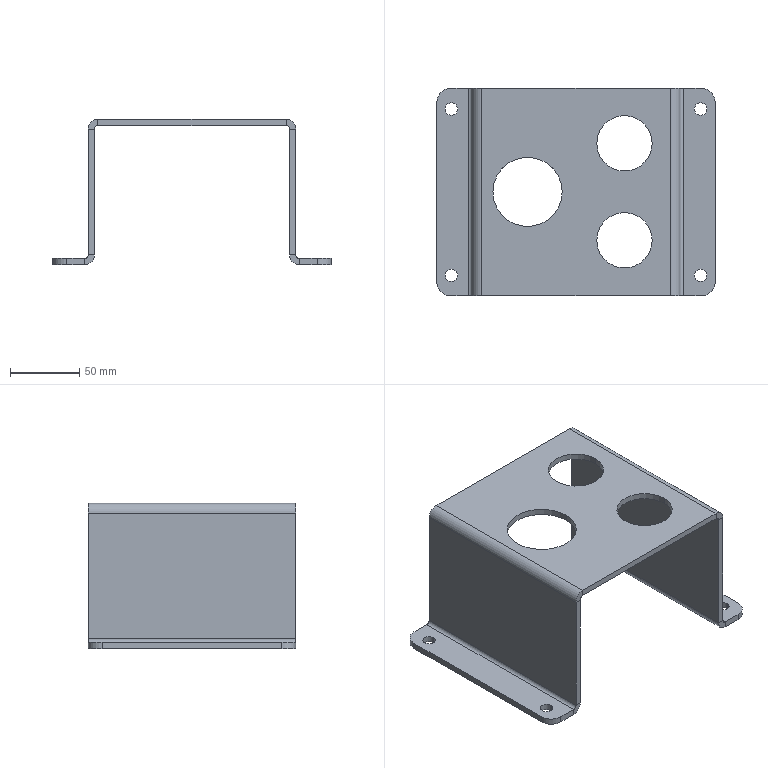Part | SolidWorks | features ICE 2, Fillet 1, FlatPattern 1, SMBaseFlange 1, SheetMetal 1, UnFold 1 | 1 solid | 56 faces | box 201 x 150 x 105 mm | volume 244169 mm3 | plane 30 | cylinder 26 | commonest cylinder face diameters 9 x8 5 x4 14 x4 20 x4 40 x4 50 x2
STEP:
#1=CARTESIAN_POINT('',(-10.,0.,0.));
#2=VERTEX_POINT('',#1);
#3=CARTESIAN_POINT('',(-60.,0.,0.));
#4=VERTEX_POINT('',#3);
#5=CARTESIAN_POINT('',(-35.,0.,0.));
#6=DIRECTION('',(0.,0.,-1.));
#7=DIRECTION('',(-1.,0.,0.));
#8=AXIS2_PLACEMENT_3D('',#5,#6,#7);
#9=CIRCLE('',#8,25.);
#10=EDGE_CURVE('',#2,#4,#9,.T.);
#11=ORIENTED_EDGE('',*,*,#10,.T.);
#12=CARTESIAN_POINT('',(-60.,0.,4.5));
#13=VERTEX_POINT('',#12);
#14=CARTESIAN_POINT('',(-60.,0.,-100.5));
#15=DIRECTION('',(0.,0.,1.));
#16=VECTOR('',#15,1000.);
#17=LINE('',#14,#16);
#18=EDGE_CURVE('',#4,#13,#17,.T.);
#19=ORIENTED_EDGE('',*,*,#18,.T.);
#20=CARTESIAN_POINT('',(-10.,0.,4.5));
#21=VERTEX_POINT('',#20);
#22=CARTESIAN_POINT('',(-35.,0.,4.5));
#23=DIRECTION('',(0.,0.,1.));
#24=DIRECTION('',(1.,0.,0.));
#25=AXIS2_PLACEMENT_3D('',#22,#23,#24);
#26=CIRCLE('',#25,25.);
#27=EDGE_CURVE('',#13,#21,#26,.T.);
#28=ORIENTED_EDGE('',*,*,#27,.T.);
#29=CARTESIAN_POINT('',(-10.,0.,-100.5));
#30=DIRECTION('',(0.,0.,1.));
#31=VECTOR('',#30,1000.);
#32=LINE('',#29,#31);
#33=EDGE_CURVE('',#2,#21,#32,.T.);
#34=ORIENTED_EDGE('',*,*,#33,.F.);
#35=EDGE_LOOP('',(#11,#19,#28,#34));
#36=FACE_OUTER_BOUND('',#35,.T.);
#37=CARTESIAN_POINT('',(-35.,0.,-100.5));
#38=DIRECTION('',(0.,0.,1.));
#39=DIRECTION('',(1.,0.,0.));
#40=AXIS2_PLACEMENT_3D('',#37,#38,#39);
#41=CYLINDRICAL_SURFACE('',#40,25.);
#42=ADVANCED_FACE('',(#36),#41,.F.);
#43=CARTESIAN_POINT('',(55.,35.,0.));
#44=VERTEX_POINT('',#43);
#45=CARTESIAN_POINT('',(15.,35.,0.));
#46=VERTEX_POINT('',#45);
#47=CARTESIAN_POINT('',(35.,35.,0.));
#48=DIRECTION('',(0.,0.,-1.));
#49=DIRECTION('',(-1.,0.,0.));
#50=AXIS2_PLACEMENT_3D('',#47,#48,#49);
#51=CIRCLE('',#50,20.);
#52=EDGE_CURVE('',#44,#46,#51,.T.);
#53=ORIENTED_EDGE('',*,*,#52,.T.);
#54=CARTESIAN_POINT('',(15.,35.,4.5));
#55=VERTEX_POINT('',#54);
#56=CARTESIAN_POINT('',(15.,35.,-100.5));
#57=DIRECTION('',(0.,0.,1.));
#58=VECTOR('',#57,1000.);
#59=LINE('',#56,#58);
#60=EDGE_CURVE('',#46,#55,#59,.T.);
#61=ORIENTED_EDGE('',*,*,#60,.T.);
#62=CARTESIAN_POINT('',(55.,35.,4.5));
#63=VERTEX_POINT('',#62);
#64=CARTESIAN_POINT('',(35.,35.,4.5));
#65=DIRECTION('',(0.,0.,1.));
#66=DIRECTION('',(1.,0.,0.));
#67=AXIS2_PLACEMENT_3D('',#64,#65,#66);
#68=CIRCLE('',#67,20.);
#69=EDGE_CURVE('',#55,#63,#68,.T.);
#70=ORIENTED_EDGE('',*,*,#69,.T.);
#71=CARTESIAN_POINT('',(55.,35.,-100.5));
#72=DIRECTION('',(0.,0.,1.));
#73=VECTOR('',#72,1000.);
#74=LINE('',#71,#73);
#75=EDGE_CURVE('',#44,#63,#74,.T.);
#76=ORIENTED_EDGE('',*,*,#75,.F.);
#77=EDGE_LOOP('',(#53,#61,#70,#76));
#78=FACE_OUTER_BOUND('',#77,.T.);
#79=CARTESIAN_POINT('',(35.,35.,-100.5));
#80=DIRECTION('',(0.,0.,1.));
#81=DIRECTION('',(1.,0.,0.));
#82=AXIS2_PLACEMENT_3D('',#79,#80,#81);
#83=CYLINDRICAL_SURFACE('',#82,20.);
#84=ADVANCED_FACE('',(#78),#83,.F.);
#85=CARTESIAN_POINT('',(55.,-35.,0.));
#86=VERTEX_POINT('',#85);
#87=CARTESIAN_POINT('',(15.,-35.,0.));
#88=VERTEX_POINT('',#87);
#89=CARTESIAN_POINT('',(35.,-35.,0.));
#90=DIRECTION('',(0.,0.,-1.));
#91=DIRECTION('',(-1.,0.,0.));
#92=AXIS2_PLACEMENT_3D('',#89,#90,#91);
#93=CIRCLE('',#92,20.);
#94=EDGE_CURVE('',#86,#88,#93,.T.);
#95=ORIENTED_EDGE('',*,*,#94,.T.);
#96=CARTESIAN_POINT('',(15.,-35.,4.5));
#97=VERTEX_POINT('',#96);
#98=CARTESIAN_POINT('',(15.,-35.,-100.5));
#99=DIRECTION('',(0.,0.,1.));
#100=VECTOR('',#99,1000.);
#101=LINE('',#98,#100);
#102=EDGE_CURVE('',#88,#97,#101,.T.);
#103=ORIENTED_EDGE('',*,*,#102,.T.);
#104=CARTESIAN_POINT('',(55.,-35.,4.5));
#105=VERTEX_POINT('',#104);
#106=CARTESIAN_POINT('',(35.,-35.,4.5));
#107=DIRECTION('',(0.,0.,1.));
#108=DIRECTION('',(1.,0.,0.));
#109=AXIS2_PLACEMENT_3D('',#106,#107,#108);
#110=CIRCLE('',#109,20.);
#111=EDGE_CURVE('',#97,#105,#110,.T.);
#112=ORIENTED_EDGE('',*,*,#111,.T.);
#113=CARTESIAN_POINT('',(55.,-35.,-100.5));
#114=DIRECTION('',(0.,0.,1.));
#115=VECTOR('',#114,1000.);
#116=LINE('',#113,#115);
#117=EDGE_CURVE('',#86,#105,#116,.T.);
#118=ORIENTED_EDGE('',*,*,#117,.F.);
#119=EDGE_LOOP('',(#95,#103,#112,#118));
#120=FACE_OUTER_BOUND('',#119,.T.);
#121=CARTESIAN_POINT('',(35.,-35.,-100.5));
#122=DIRECTION('',(0.,0.,1.));
#123=DIRECTION('',(1.,0.,0.));
#124=AXIS2_PLACEMENT_3D('',#121,#122,#123);
#125=CYLINDRICAL_SURFACE('',#124,20.);
#126=ADVANCED_FACE('',(#120),#125,.F.);
#127=CARTESIAN_POINT('',(85.5,-60.,-100.5));
#128=VERTEX_POINT('',#127);
#129=CARTESIAN_POINT('',(94.5,-60.,-100.5));
#130=VERTEX_POINT('',#129);
#131=CARTESIAN_POINT('',(90.,-60.,-100.5));
#132=DIRECTION('',(0.,0.,1.));
#133=DIRECTION('',(1.,0.,0.));
#134=AXIS2_PLACEMENT_3D('',#131,#132,#133);
#135=CIRCLE('',#134,4.5);
#136=EDGE_CURVE('',#128,#130,#135,.T.);
#137=ORIENTED_EDGE('',*,*,#136,.F.);
#138=CARTESIAN_POINT('',(85.5,-60.,-96.));
#139=VERTEX_POINT('',#138);
#140=CARTESIAN_POINT('',(85.5,-60.,-100.5));
#141=DIRECTION('',(0.,0.,1.));
#142=VECTOR('',#141,1000.);
#143=LINE('',#140,#142);
#144=EDGE_CURVE('',#128,#139,#143,.T.);
#145=ORIENTED_EDGE('',*,*,#144,.T.);
#146=CARTESIAN_POINT('',(94.5,-60.,-96.));
#147=VERTEX_POINT('',#146);
#148=CARTESIAN_POINT('',(90.,-60.,-96.));
#149=DIRECTION('',(0.,0.,-1.));
#150=DIRECTION('',(-1.,0.,0.));
#151=AXIS2_PLACEMENT_3D('',#148,#149,#150);
#152=CIRCLE('',#151,4.5);
#153=EDGE_CURVE('',#147,#139,#152,.T.);
#154=ORIENTED_EDGE('',*,*,#153,.F.);
#155=CARTESIAN_POINT('',(94.5,-60.,-100.5));
#156=DIRECTION('',(0.,0.,1.));
#157=VECTOR('',#156,1000.);
#158=LINE('',#155,#157);
#159=EDGE_CURVE('',#130,#147,#158,.T.);
#160=ORIENTED_EDGE('',*,*,#159,.F.);
#161=EDGE_LOOP('',(#137,#145,#154,#160));
#162=FACE_OUTER_BOUND('',#161,.T.);
#163=CARTESIAN_POINT('',(90.,-60.,-100.5));
#164=DIRECTION('',(0.,0.,1.));
#165=DIRECTION('',(1.,0.,0.));
#166=AXIS2_PLACEMENT_3D('',#163,#164,#165);
#167=CYLINDRICAL_SURFACE('',#166,4.5);
#168=ADVANCED_FACE('',(#162),#167,.F.);
#169=CARTESIAN_POINT('',(85.5,60.,-100.5));
#170=VERTEX_POINT('',#169);
#171=CARTESIAN_POINT('',(94.5,60.,-100.5));
#172=VERTEX_POINT('',#171);
#173=CARTESIAN_POINT('',(90.,60.,-100.5));
#174=DIRECTION('',(0.,0.,1.));
#175=DIRECTION('',(1.,0.,0.));
#176=AXIS2_PLACEMENT_3D('',#173,#174,#175);
#177=CIRCLE('',#176,4.5);
#178=EDGE_CURVE('',#170,#172,#177,.T.);
#179=ORIENTED_EDGE('',*,*,#178,.F.);
#180=CARTESIAN_POINT('',(85.5,60.,-96.));
#181=VERTEX_POINT('',#180);
#182=CARTESIAN_POINT('',(85.5,60.,-100.5));
#183=DIRECTION('',(0.,0.,1.));
#184=VECTOR('',#183,1000.);
#185=LINE('',#182,#184);
#186=EDGE_CURVE('',#170,#181,#185,.T.);
#187=ORIENTED_EDGE('',*,*,#186,.T.);
#188=CARTESIAN_POINT('',(94.5,60.,-96.));
#189=VERTEX_POINT('',#188);
#190=CARTESIAN_POINT('',(90.,60.,-96.));
#191=DIRECTION('',(0.,0.,-1.));
#192=DIRECTION('',(-1.,0.,0.));
#193=AXIS2_PLACEMENT_3D('',#190,#191,#192);
#194=CIRCLE('',#193,4.5);
#195=EDGE_CURVE('',#189,#181,#194,.T.);
#196=ORIENTED_EDGE('',*,*,#195,.F.);
#197=CARTESIAN_POINT('',(94.5,60.,-100.5));
#198=DIRECTION('',(0.,0.,1.));
#199=VECTOR('',#198,1000.);
#200=LINE('',#197,#199);
#201=EDGE_CURVE('',#172,#189,#200,.T.);
#202=ORIENTED_EDGE('',*,*,#201,.F.);
#203=EDGE_LOOP('',(#179,#187,#196,#202));
#204=FACE_OUTER_BOUND('',#203,.T.);
#205=CARTESIAN_POINT('',(90.,60.,-100.5));
#206=DIRECTION('',(0.,0.,1.));
#207=DIRECTION('',(1.,0.,0.));
#208=AXIS2_PLACEMENT_3D('',#205,#206,#207);
#209=CYLINDRICAL_SURFACE('',#208,4.5);
#210=ADVANCED_FACE('',(#204),#209,.F.);
#211=CARTESIAN_POINT('',(-94.5,-60.,-100.5));
#212=VERTEX_POINT('',#211);
#213=CARTESIAN_POINT('',(-85.5,-60.,-100.5));
#214=VERTEX_POINT('',#213);
#215=CARTESIAN_POINT('',(-90.,-60.,-100.5));
#216=DIRECTION('',(0.,0.,1.));
#217=DIRECTION('',(1.,0.,0.));
#218=AXIS2_PLACEMENT_3D('',#215,#216,#217);
#219=CIRCLE('',#218,4.5);
#220=EDGE_CURVE('',#212,#214,#219,.T.);
#221=ORIENTED_EDGE('',*,*,#220,.F.);
#222=CARTESIAN_POINT('',(-94.5,-60.,-96.));
#223=VERTEX_POINT('',#222);
#224=CARTESIAN_POINT('',(-94.5,-60.,-100.5));
#225=DIRECTION('',(0.,0.,1.));
#226=VECTOR('',#225,1000.);
#227=LINE('',#224,#226);
#228=EDGE_CURVE('',#212,#223,#227,.T.);
#229=ORIENTED_EDGE('',*,*,#228,.T.);
#230=CARTESIAN_POINT('',(-85.5,-60.,-96.));
#231=VERTEX_POINT('',#230);
#232=CARTESIAN_POINT('',(-90.,-60.,-96.));
#233=DIRECTION('',(0.,0.,-1.));
#234=DIRECTION('',(-1.,0.,0.));
#235=AXIS2_PLACEMENT_3D('',#232,#233,#234);
#236=CIRCLE('',#235,4.5);
#237=EDGE_CURVE('',#231,#223,#236,.T.);
#238=ORIENTED_EDGE('',*,*,#237,.F.);
#239=CARTESIAN_POINT('',(-85.5,-60.,-100.5));
#240=DIRECTION('',(0.,0.,1.));
#241=VECTOR('',#240,1000.);
#242=LINE('',#239,#241);
#243=EDGE_CURVE('',#214,#231,#242,.T.);
#244=ORIENTED_EDGE('',*,*,#243,.F.);
#245=EDGE_LOOP('',(#221,#229,#238,#244));
#246=FACE_OUTER_BOUND('',#245,.T.);
#247=CARTESIAN_POINT('',(-90.,-60.,-100.5));
#248=DIRECTION('',(0.,0.,1.));
#249=DIRECTION('',(1.,0.,0.));
#250=AXIS2_PLACEMENT_3D('',#247,#248,#249);
#251=CYLINDRICAL_SURFACE('',#250,4.5);
#252=ADVANCED_FACE('',(#246),#251,.F.);
#253=CARTESIAN_POINT('',(-94.5,60.,-100.5));
#254=VERTEX_POINT('',#253);
#255=CARTESIAN_POINT('',(-85.5,60.,-100.5));
#256=VERTEX_POINT('',#255);
#257=CARTESIAN_POINT('',(-90.,60.,-100.5));
#258=DIRECTION('',(0.,0.,1.));
#259=DIRECTION('',(1.,0.,0.));
#260=AXIS2_PLACEMENT_3D('',#257,#258,#259);
#261=CIRCLE('',#260,4.5);
#262=EDGE_CURVE('',#254,#256,#261,.T.);
#263=ORIENTED_EDGE('',*,*,#262,.F.);
#264=CARTESIAN_POINT('',(-94.5,60.,-96.));
#265=VERTEX_POINT('',#264);
#266=CARTESIAN_POINT('',(-94.5,60.,-100.5));
#267=DIRECTION('',(0.,0.,1.));
#268=VECTOR('',#267,1000.);
#269=LINE('',#266,#268);
#270=EDGE_CURVE('',#254,#265,#269,.T.);
#271=ORIENTED_EDGE('',*,*,#270,.T.);
#272=CARTESIAN_POINT('',(-85.5,60.,-96.));
#273=VERTEX_POINT('',#272);
#274=CARTESIAN_POINT('',(-90.,60.,-96.));
#275=DIRECTION('',(0.,0.,-1.));
#276=DIRECTION('',(-1.,0.,0.));
#277=AXIS2_PLACEMENT_3D('',#274,#275,#276);
#278=CIRCLE('',#277,4.5);
#279=EDGE_CURVE('',#273,#265,#278,.T.);
#280=ORIENTED_EDGE('',*,*,#279,.F.);
#281=CARTESIAN_POINT('',(-85.5,60.,-100.5));
#282=DIRECTION('',(0.,0.,1.));
#283=VECTOR('',#282,1000.);
#284=LINE('',#281,#283);
#285=EDGE_CURVE('',#256,#273,#284,.T.);
#286=ORIENTED_EDGE('',*,*,#285,.F.);
#287=EDGE_LOOP('',(#263,#271,#280,#286));
#288=FACE_OUTER_BOUND('',#287,.T.);
#289=CARTESIAN_POINT('',(-90.,60.,-100.5));
#290=DIRECTION('',(0.,0.,1.));
#291=DIRECTION('',(1.,0.,0.));
#292=AXIS2_PLACEMENT_3D('',#289,#290,#291);
#293=CYLINDRICAL_SURFACE('',#292,4.5);
#294=ADVANCED_FACE('',(#288),#293,.F.);
#295=CARTESIAN_POINT('',(77.5,75.,-100.5));
#296=VERTEX_POINT('',#295);
#297=CARTESIAN_POINT('',(77.5,75.,-96.));
#298=VERTEX_POINT('',#297);
#299=CARTESIAN_POINT('',(77.5,75.,-100.5));
#300=DIRECTION('',(0.,0.,1.));
#301=VECTOR('',#300,1000.);
#302=LINE('',#299,#301);
#303=EDGE_CURVE('',#296,#298,#302,.T.);
#304=ORIENTED_EDGE('',*,*,#303,.F.);
#305=CARTESIAN_POINT('',(70.5,75.,-93.5));
#306=VERTEX_POINT('',#305);
#307=CARTESIAN_POINT('',(77.5,75.,-93.5));
#308=DIRECTION('',(0.,-1.,0.));
#309=DIRECTION('',(0.,0.,-1.));
#310=AXIS2_PLACEMENT_3D('',#307,#308,#309);
#311=CIRCLE('',#310,7.);
#312=EDGE_CURVE('',#306,#296,#311,.T.);
#313=ORIENTED_EDGE('',*,*,#312,.F.);
#314=CARTESIAN_POINT('',(75.,75.,-93.5));
#315=VERTEX_POINT('',#314);
#316=CARTESIAN_POINT('',(75.,75.,-93.5));
#317=DIRECTION('',(-1.,0.,0.));
#318=VECTOR('',#317,1000.);
#319=LINE('',#316,#318);
#320=EDGE_CURVE('',#315,#306,#319,.T.);
#321=ORIENTED_EDGE('',*,*,#320,.F.);
#322=CARTESIAN_POINT('',(77.5,75.,-93.5));
#323=DIRECTION('',(0.,-1.,0.));
#324=DIRECTION('',(1.,0.,0.));
#325=AXIS2_PLACEMENT_3D('',#322,#323,#324);
#326=CIRCLE('',#325,2.5);
#327=EDGE_CURVE('',#315,#298,#326,.T.);
#328=ORIENTED_EDGE('',*,*,#327,.T.);
#329=EDGE_LOOP('',(#304,#313,#321,#328));
#330=FACE_OUTER_BOUND('',#329,.T.);
#331=CARTESIAN_POINT('',(77.5,75.,-100.5));
#332=DIRECTION('',(0.,1.,0.));
#333=DIRECTION('',(0.,0.,1.));
#334=AXIS2_PLACEMENT_3D('',#331,#332,#333);
#335=PLANE('',#334);
#336=ADVANCED_FACE('',(#330),#335,.T.);
#337=CARTESIAN_POINT('',(90.5,75.,-96.));
#338=VERTEX_POINT('',#337);
#339=CARTESIAN_POINT('',(70.5,75.,-96.));
#340=DIRECTION('',(1.,0.,0.));
#341=VECTOR('',#340,1000.);
#342=LINE('',#339,#341);
#343=EDGE_CURVE('',#298,#338,#342,.T.);
#344=ORIENTED_EDGE('',*,*,#343,.T.);
#345=CARTESIAN_POINT('',(90.5,75.,-100.5));
#346=VERTEX_POINT('',#345);
#347=CARTESIAN_POINT('',(90.5,75.,-93.5));
#348=DIRECTION('',(0.,0.,-1.));
#349=VECTOR('',#348,1000.);
#350=LINE('',#347,#349);
#351=EDGE_CURVE('',#338,#346,#350,.T.);
#352=ORIENTED_EDGE('',*,*,#351,.T.);
#353=CARTESIAN_POINT('',(70.5,75.,-100.5));
#354=DIRECTION('',(1.,0.,0.));
#355=VECTOR('',#354,1000.);
#356=LINE('',#353,#355);
#357=EDGE_CURVE('',#296,#346,#356,.T.);
#358=ORIENTED_EDGE('',*,*,#357,.F.);
#359=ORIENTED_EDGE('',*,*,#303,.T.);
#360=EDGE_LOOP('',(#344,#352,#358,#359));
#361=FACE_OUTER_BOUND('',#360,.T.);
#362=CARTESIAN_POINT('',(75.,75.,-93.5));
#363=DIRECTION('',(0.,1.,0.));
#364=DIRECTION('',(0.,0.,1.));
#365=AXIS2_PLACEMENT_3D('',#362,#363,#364);
#366=PLANE('',#365);
#367=ADVANCED_FACE('',(#361),#366,.T.);
#368=CARTESIAN_POINT('',(70.5,-75.,-93.5));
#369=VERTEX_POINT('',#368);
#370=CARTESIAN_POINT('',(75.,-75.,-93.5));
#371=VERTEX_POINT('',#370);
#372=CARTESIAN_POINT('',(70.5,-75.,-93.5));
#373=DIRECTION('',(1.,0.,0.));
#374=VECTOR('',#373,1000.);
#375=LINE('',#372,#374);
#376=EDGE_CURVE('',#369,#371,#375,.T.);
#377=ORIENTED_EDGE('',*,*,#376,.F.);
#378=CARTESIAN_POINT('',(77.5,-75.,-100.5));
#379=VERTEX_POINT('',#378);
#380=CARTESIAN_POINT('',(77.5,-75.,-93.5));
#381=DIRECTION('',(0.,-1.,0.));
#382=DIRECTION('',(0.,0.,-1.));
#383=AXIS2_PLACEMENT_3D('',#380,#381,#382);
#384=CIRCLE('',#383,7.);
#385=EDGE_CURVE('',#369,#379,#384,.T.);
#386=ORIENTED_EDGE('',*,*,#385,.T.);
#387=CARTESIAN_POINT('',(77.5,-75.,-96.));
#388=VERTEX_POINT('',#387);
#389=CARTESIAN_POINT('',(77.5,-75.,-96.));
#390=DIRECTION('',(0.,0.,-1.));
#391=VECTOR('',#390,1000.);
#392=LINE('',#389,#391);
#393=EDGE_CURVE('',#388,#379,#392,.T.);
#394=ORIENTED_EDGE('',*,*,#393,.F.);
#395=CARTESIAN_POINT('',(77.5,-75.,-93.5));
#396=DIRECTION('',(0.,-1.,0.));
#397=DIRECTION('',(1.,0.,0.));
#398=AXIS2_PLACEMENT_3D('',#395,#396,#397);
#399=CIRCLE('',#398,2.5);
#400=EDGE_CURVE('',#371,#388,#399,.T.);
#401=ORIENTED_EDGE('',*,*,#400,.F.);
#402=EDGE_LOOP('',(#377,#386,#394,#401));
#403=FACE_OUTER_BOUND('',#402,.T.);
#404=CARTESIAN_POINT('',(70.5,-75.,-93.5));
#405=DIRECTION('',(0.,-1.,0.));
#406=DIRECTION('',(0.,0.,-1.));
#407=AXIS2_PLACEMENT_3D('',#404,#405,#406);
#408=PLANE('',#407);
#409=ADVANCED_FACE('',(#403),#408,.T.);
#410=CARTESIAN_POINT('',(70.5,-75.,-2.5));
#411=VERTEX_POINT('',#410);
#412=CARTESIAN_POINT('',(70.5,-75.,0.));
#413=DIRECTION('',(0.,0.,-1.));
#414=VECTOR('',#413,1000.);
#415=LINE('',#412,#414);
#416=EDGE_CURVE('',#411,#369,#415,.T.);
#417=ORIENTED_EDGE('',*,*,#416,.T.);
#418=ORIENTED_EDGE('',*,*,#376,.T.);
#419=CARTESIAN_POINT('',(75.,-75.,-2.5));
#420=VERTEX_POINT('',#419);
#421=CARTESIAN_POINT('',(75.,-75.,0.));
#422=DIRECTION('',(0.,0.,-1.));
#423=VECTOR('',#422,1000.);
#424=LINE('',#421,#423);
#425=EDGE_CURVE('',#420,#371,#424,.T.);
#426=ORIENTED_EDGE('',*,*,#425,.F.);
#427=CARTESIAN_POINT('',(75.,-75.,-2.5));
#428=DIRECTION('',(-1.,0.,0.));
#429=VECTOR('',#428,1000.);
#430=LINE('',#427,#429);
#431=EDGE_CURVE('',#420,#411,#430,.T.);
#432=ORIENTED_EDGE('',*,*,#431,.T.);
#433=EDGE_LOOP('',(#417,#418,#426,#432));
#434=FACE_OUTER_BOUND('',#433,.T.);
#435=CARTESIAN_POINT('',(77.5,-75.,-96.));
#436=DIRECTION('',(0.,-1.,0.));
#437=DIRECTION('',(0.,0.,-1.));
#438=AXIS2_PLACEMENT_3D('',#435,#436,#437);
#439=PLANE('',#438);
#440=ADVANCED_FACE('',(#434),#439,.T.);
#441=CARTESIAN_POINT('',(70.5,75.,-2.5));
#442=VERTEX_POINT('',#441);
#443=CARTESIAN_POINT('',(75.,75.,-2.5));
#444=VERTEX_POINT('',#443);
#445=CARTESIAN_POINT('',(70.5,75.,-2.5));
#446=DIRECTION('',(1.,0.,0.));
#447=VECTOR('',#446,1000.);
#448=LINE('',#445,#447);
#449=EDGE_CURVE('',#442,#444,#448,.T.);
#450=ORIENTED_EDGE('',*,*,#449,.F.);
#451=CARTESIAN_POINT('',(68.,75.,0.));
#452=VERTEX_POINT('',#451);
#453=CARTESIAN_POINT('',(68.,75.,-2.5));
#454=DIRECTION('',(0.,1.,0.));
#455=DIRECTION('',(0.,0.,1.));
#456=AXIS2_PLACEMENT_3D('',#453,#454,#455);
#457=CIRCLE('',#456,2.5);
#458=EDGE_CURVE('',#452,#442,#457,.T.);
#459=ORIENTED_EDGE('',*,*,#458,.F.);
#460=CARTESIAN_POINT('',(68.,75.,4.5));
#461=VERTEX_POINT('',#460);
#462=CARTESIAN_POINT('',(68.,75.,4.5));
#463=DIRECTION('',(0.,0.,-1.));
#464=VECTOR('',#463,1000.);
#465=LINE('',#462,#464);
#466=EDGE_CURVE('',#461,#452,#465,.T.);
#467=ORIENTED_EDGE('',*,*,#466,.F.);
#468=CARTESIAN_POINT('',(68.,75.,-2.5));
#469=DIRECTION('',(0.,1.,0.));
#470=DIRECTION('',(1.,0.,0.));
#471=AXIS2_PLACEMENT_3D('',#468,#469,#470);
#472=CIRCLE('',#471,7.);
#473=EDGE_CURVE('',#461,#444,#472,.T.);
#474=ORIENTED_EDGE('',*,*,#473,.T.);
#475=EDGE_LOOP('',(#450,#459,#467,#474));
#476=FACE_OUTER_BOUND('',#475,.T.);
#477=CARTESIAN_POINT('',(70.5,75.,-2.5));
#478=DIRECTION('',(0.,1.,0.));
#479=DIRECTION('',(0.,0.,1.));
#480=AXIS2_PLACEMENT_3D('',#477,#478,#479);
#481=PLANE('',#480);
#482=ADVANCED_FACE('',(#476),#481,.T.);
#483=CARTESIAN_POINT('',(70.5,75.,0.));
#484=DIRECTION('',(0.,0.,-1.));
#485=VECTOR('',#484,1000.);
#486=LINE('',#483,#485);
#487=EDGE_CURVE('',#442,#306,#486,.T.);
#488=ORIENTED_EDGE('',*,*,#487,.F.);
#489=ORIENTED_EDGE('',*,*,#449,.T.);
#490=CARTESIAN_POINT('',(75.,75.,0.));
#491=DIRECTION('',(0.,0.,-1.));
#492=VECTOR('',#491,1000.);
#493=LINE('',#490,#492);
#494=EDGE_CURVE('',#444,#315,#493,.T.);
#495=ORIENTED_EDGE('',*,*,#494,.T.);
#496=ORIENTED_EDGE('',*,*,#320,.T.);
#497=EDGE_LOOP('',(#488,#489,#495,#496));
#498=FACE_OUTER_BOUND('',#497,.T.);
#499=CARTESIAN_POINT('',(68.,75.,4.5));
#500=DIRECTION('',(0.,1.,0.));
#501=DIRECTION('',(0.,0.,1.));
#502=AXIS2_PLACEMENT_3D('',#499,#500,#501);
#503=PLANE('',#502);
#504=ADVANCED_FACE('',(#498),#503,.T.);
#505=CARTESIAN_POINT('',(68.,-75.,0.));
#506=VERTEX_POINT('',#505);
#507=CARTESIAN_POINT('',(68.,-75.,4.5));
#508=VERTEX_POINT('',#507);
#509=CARTESIAN_POINT('',(68.,-75.,0.));
#510=DIRECTION('',(0.,0.,1.));
#511=VECTOR('',#510,1000.);
#512=LINE('',#509,#511);
#513=EDGE_CURVE('',#506,#508,#512,.T.);
#514=ORIENTED_EDGE('',*,*,#513,.F.);
#515=CARTESIAN_POINT('',(68.,-75.,-2.5));
#516=DIRECTION('',(0.,1.,0.));
#517=DIRECTION('',(0.,0.,1.));
#518=AXIS2_PLACEMENT_3D('',#515,#516,#517);
#519=CIRCLE('',#518,2.5);
#520=EDGE_CURVE('',#506,#411,#519,.T.);
#521=ORIENTED_EDGE('',*,*,#520,.T.);
#522=ORIENTED_EDGE('',*,*,#431,.F.);
#523=CARTESIAN_POINT('',(68.,-75.,-2.5));
#524=DIRECTION('',(0.,1.,0.));
#525=DIRECTION('',(1.,0.,0.));
#526=AXIS2_PLACEMENT_3D('',#523,#524,#525);
#527=CIRCLE('',#526,7.);
#528=EDGE_CURVE('',#508,#420,#527,.T.);
#529=ORIENTED_EDGE('',*,*,#528,.F.);
#530=EDGE_LOOP('',(#514,#521,#522,#529));
#531=FACE_OUTER_BOUND('',#530,.T.);
#532=CARTESIAN_POINT('',(68.,-75.,0.));
#533=DIRECTION('',(0.,-1.,0.));
#534=DIRECTION('',(0.,0.,-1.));
#535=AXIS2_PLACEMENT_3D('',#532,#533,#534);
#536=PLANE('',#535);
#537=ADVANCED_FACE('',(#531),#536,.T.);
#538=CARTESIAN_POINT('',(-68.,-75.,0.));
#539=VERTEX_POINT('',#538);
#540=CARTESIAN_POINT('',(-70.5,-75.,0.));
#541=DIRECTION('',(1.,0.,0.));
#542=VECTOR('',#541,1000.);
#543=LINE('',#540,#542);
#544=EDGE_CURVE('',#539,#506,#543,.T.);
#545=ORIENTED_EDGE('',*,*,#544,.T.);
#546=ORIENTED_EDGE('',*,*,#513,.T.);
#547=CARTESIAN_POINT('',(-68.,-75.,4.5));
#548=VERTEX_POINT('',#547);
#549=CARTESIAN_POINT('',(-70.5,-75.,4.5));
#550=DIRECTION('',(1.,0.,0.));
#551=VECTOR('',#550,1000.);
#552=LINE('',#549,#551);
#553=EDGE_CURVE('',#548,#508,#552,.T.);
#554=ORIENTED_EDGE('',*,*,#553,.F.);
#555=CARTESIAN_POINT('',(-68.,-75.,4.5));
#556=DIRECTION('',(0.,0.,-1.));
#557=VECTOR('',#556,1000.);
#558=LINE('',#555,#557);
#559=EDGE_CURVE('',#548,#539,#558,.T.);
#560=ORIENTED_EDGE('',*,*,#559,.T.);
#561=EDGE_LOOP('',(#545,#546,#554,#560));
#562=FACE_OUTER_BOUND('',#561,.T.);
#563=CARTESIAN_POINT('',(75.,-75.,-2.5));
#564=DIRECTION('',(0.,-1.,0.));
#565=DIRECTION('',(0.,0.,-1.));
#566=AXIS2_PLACEMENT_3D('',#563,#564,#565);
#567=PLANE('',#566);
#568=ADVANCED_FACE('',(#562),#567,.T.);
#569=CARTESIAN_POINT('',(-68.,75.,0.));
#570=VERTEX_POINT('',#569);
#571=CARTESIAN_POINT('',(-68.,75.,4.5));
#572=VERTEX_POINT('',#571);
#573=CARTESIAN_POINT('',(-68.,75.,0.));
#574=DIRECTION('',(0.,0.,1.));
#575=VECTOR('',#574,1000.);
#576=LINE('',#573,#575);
#577=EDGE_CURVE('',#570,#572,#576,.T.);
#578=ORIENTED_EDGE('',*,*,#577,.F.);
#579=CARTESIAN_POINT('',(-70.5,75.,-2.5));
#580=VERTEX_POINT('',#579);
#581=CARTESIAN_POINT('',(-68.,75.,-2.5));
#582=DIRECTION('',(0.,1.,0.));
#583=DIRECTION('',(0.,0.,1.));
#584=AXIS2_PLACEMENT_3D('',#581,#582,#583);
#585=CIRCLE('',#584,2.5);
#586=EDGE_CURVE('',#580,#570,#585,.T.);
#587=ORIENTED_EDGE('',*,*,#586,.F.);
#588=CARTESIAN_POINT('',(-75.,75.,-2.5));
#589=VERTEX_POINT('',#588);
#590=CARTESIAN_POINT('',(-75.,75.,-2.5));
#591=DIRECTION('',(1.,0.,0.));
#592=VECTOR('',#591,1000.);
#593=LINE('',#590,#592);
#594=EDGE_CURVE('',#589,#580,#593,.T.);
#595=ORIENTED_EDGE('',*,*,#594,.F.);
#596=CARTESIAN_POINT('',(-68.,75.,-2.5));
#597=DIRECTION('',(0.,1.,0.));
#598=DIRECTION('',(1.,0.,0.));
#599=AXIS2_PLACEMENT_3D('',#596,#597,#598);
#600=CIRCLE('',#599,7.);
#601=EDGE_CURVE('',#589,#572,#600,.T.);
#602=ORIENTED_EDGE('',*,*,#601,.T.);
#603=EDGE_LOOP('',(#578,#587,#595,#602));
#604=FACE_OUTER_BOUND('',#603,.T.);
#605=CARTESIAN_POINT('',(-68.,75.,0.));
#606=DIRECTION('',(0.,1.,0.));
#607=DIRECTION('',(0.,0.,1.));
#608=AXIS2_PLACEMENT_3D('',#605,#606,#607);
#609=PLANE('',#608);
#610=ADVANCED_FACE('',(#604),#609,.T.);
#611=CARTESIAN_POINT('',(-70.5,75.,0.));
#612=DIRECTION('',(1.,0.,0.));
#613=VECTOR('',#612,1000.);
#614=LINE('',#611,#613);
#615=EDGE_CURVE('',#570,#452,#614,.T.);
#616=ORIENTED_EDGE('',*,*,#615,.F.);
#617=ORIENTED_EDGE('',*,*,#577,.T.);
#618=CARTESIAN_POINT('',(-70.5,75.,4.5));
#619=DIRECTION('',(1.,0.,0.));
#620=VECTOR('',#619,1000.);
#621=LINE('',#618,#620);
#622=EDGE_CURVE('',#572,#461,#621,.T.);
#623=ORIENTED_EDGE('',*,*,#622,.T.);
#624=ORIENTED_EDGE('',*,*,#466,.T.);
#625=EDGE_LOOP('',(#616,#617,#623,#624));
#626=FACE_OUTER_BOUND('',#625,.T.);
#627=CARTESIAN_POINT('',(-75.,75.,-2.5));
#628=DIRECTION('',(0.,1.,0.));
#629=DIRECTION('',(0.,0.,1.));
#630=AXIS2_PLACEMENT_3D('',#627,#628,#629);
#631=PLANE('',#630);
#632=ADVANCED_FACE('',(#626),#631,.T.);
#633=CARTESIAN_POINT('',(-70.5,-75.,-2.5));
#634=VERTEX_POINT('',#633);
#635=CARTESIAN_POINT('',(-75.,-75.,-2.5));
#636=VERTEX_POINT('',#635);
#637=CARTESIAN_POINT('',(-70.5,-75.,-2.5));
#638=DIRECTION('',(-1.,0.,0.));
#639=VECTOR('',#638,1000.);
#640=LINE('',#637,#639);
#641=EDGE_CURVE('',#634,#636,#640,.T.);
#642=ORIENTED_EDGE('',*,*,#641,.F.);
#643=CARTESIAN_POINT('',(-68.,-75.,-2.5));
#644=DIRECTION('',(0.,1.,0.));
#645=DIRECTION('',(0.,0.,1.));
#646=AXIS2_PLACEMENT_3D('',#643,#644,#645);
#647=CIRCLE('',#646,2.5);
#648=EDGE_CURVE('',#634,#539,#647,.T.);
#649=ORIENTED_EDGE('',*,*,#648,.T.);
#650=ORIENTED_EDGE('',*,*,#559,.F.);
#651=CARTESIAN_POINT('',(-68.,-75.,-2.5));
#652=DIRECTION('',(0.,1.,0.));
#653=DIRECTION('',(1.,0.,0.));
#654=AXIS2_PLACEMENT_3D('',#651,#652,#653);
#655=CIRCLE('',#654,7.);
#656=EDGE_CURVE('',#636,#548,#655,.T.);
#657=ORIENTED_EDGE('',*,*,#656,.F.);
#658=EDGE_LOOP('',(#642,#649,#650,#657));
#659=FACE_OUTER_BOUND('',#658,.T.);
#660=CARTESIAN_POINT('',(-70.5,-75.,-2.5));
#661=DIRECTION('',(0.,-1.,0.));
#662=DIRECTION('',(0.,0.,-1.));
#663=AXIS2_PLACEMENT_3D('',#660,#661,#662);
#664=PLANE('',#663);
#665=ADVANCED_FACE('',(#659),#664,.T.);
#666=CARTESIAN_POINT('',(-70.5,-75.,-93.5));
#667=VERTEX_POINT('',#666);
#668=CARTESIAN_POINT('',(-70.5,-75.,0.));
#669=DIRECTION('',(0.,0.,1.));
#670=VECTOR('',#669,1000.);
#671=LINE('',#668,#670);
#672=EDGE_CURVE('',#667,#634,#671,.T.);
#673=ORIENTED_EDGE('',*,*,#672,.T.);
#674=ORIENTED_EDGE('',*,*,#641,.T.);
#675=CARTESIAN_POINT('',(-75.,-75.,-93.5));
#676=VERTEX_POINT('',#675);
#677=CARTESIAN_POINT('',(-75.,-75.,0.));
#678=DIRECTION('',(0.,0.,1.));
#679=VECTOR('',#678,1000.);
#680=LINE('',#677,#679);
#681=EDGE_CURVE('',#676,#636,#680,.T.);
#682=ORIENTED_EDGE('',*,*,#681,.F.);
#683=CARTESIAN_POINT('',(-75.,-75.,-93.5));
#684=DIRECTION('',(1.,0.,0.));
#685=VECTOR('',#684,1000.);
#686=LINE('',#683,#685);
#687=EDGE_CURVE('',#676,#667,#686,.T.);
#688=ORIENTED_EDGE('',*,*,#687,.T.);
#689=EDGE_LOOP('',(#673,#674,#682,#688));
#690=FACE_OUTER_BOUND('',#689,.T.);
#691=CARTESIAN_POINT('',(-68.,-75.,4.5));
#692=DIRECTION('',(0.,-1.,0.));
#693=DIRECTION('',(0.,0.,-1.));
#694=AXIS2_PLACEMENT_3D('',#691,#692,#693);
#695=PLANE('',#694);
#696=ADVANCED_FACE('',(#690),#695,.T.);
#697=CARTESIAN_POINT('',(-70.5,75.,-93.5));
#698=VERTEX_POINT('',#697);
#699=CARTESIAN_POINT('',(-75.,75.,-93.5));
#700=VERTEX_POINT('',#699);
#701=CARTESIAN_POINT('',(-70.5,75.,-93.5));
#702=DIRECTION('',(-1.,0.,0.));
#703=VECTOR('',#702,1000.);
#704=LINE('',#701,#703);
#705=EDGE_CURVE('',#698,#700,#704,.T.);
#706=ORIENTED_EDGE('',*,*,#705,.F.);
#707=CARTESIAN_POINT('',(-77.5,75.,-100.5));
#708=VERTEX_POINT('',#707);
#709=CARTESIAN_POINT('',(-77.5,75.,-93.5));
#710=DIRECTION('',(0.,-1.,0.));
#711=DIRECTION('',(0.,0.,-1.));
#712=AXIS2_PLACEMENT_3D('',#709,#710,#711);
#713=CIRCLE('',#712,7.);
#714=EDGE_CURVE('',#708,#698,#713,.T.);
#715=ORIENTED_EDGE('',*,*,#714,.F.);
#716=CARTESIAN_POINT('',(-77.5,75.,-96.));
#717=VERTEX_POINT('',#716);
#718=CARTESIAN_POINT('',(-77.5,75.,-96.));
#719=DIRECTION('',(0.,0.,-1.));
#720=VECTOR('',#719,1000.);
#721=LINE('',#718,#720);
#722=EDGE_CURVE('',#717,#708,#721,.T.);
#723=ORIENTED_EDGE('',*,*,#722,.F.);
#724=CARTESIAN_POINT('',(-77.5,75.,-93.5));
#725=DIRECTION('',(0.,-1.,0.));
#726=DIRECTION('',(1.,0.,0.));
#727=AXIS2_PLACEMENT_3D('',#724,#725,#726);
#728=CIRCLE('',#727,2.5);
#729=EDGE_CURVE('',#717,#700,#728,.T.);
#730=ORIENTED_EDGE('',*,*,#729,.T.);
#731=EDGE_LOOP('',(#706,#715,#723,#730));
#732=FACE_OUTER_BOUND('',#731,.T.);
#733=CARTESIAN_POINT('',(-70.5,75.,-93.5));
#734=DIRECTION('',(0.,1.,0.));
#735=DIRECTION('',(0.,0.,1.));
#736=AXIS2_PLACEMENT_3D('',#733,#734,#735);
#737=PLANE('',#736);
#738=ADVANCED_FACE('',(#732),#737,.T.);
#739=CARTESIAN_POINT('',(-70.5,75.,0.));
#740=DIRECTION('',(0.,0.,1.));
#741=VECTOR('',#740,1000.);
#742=LINE('',#739,#741);
#743=EDGE_CURVE('',#698,#580,#742,.T.);
#744=ORIENTED_EDGE('',*,*,#743,.F.);
#745=ORIENTED_EDGE('',*,*,#705,.T.);
#746=CARTESIAN_POINT('',(-75.,75.,0.));
#747=DIRECTION('',(0.,0.,1.));
#748=VECTOR('',#747,1000.);
#749=LINE('',#746,#748);
#750=EDGE_CURVE('',#700,#589,#749,.T.);
#751=ORIENTED_EDGE('',*,*,#750,.T.);
#752=ORIENTED_EDGE('',*,*,#594,.T.);
#753=EDGE_LOOP('',(#744,#745,#751,#752));
#754=FACE_OUTER_BOUND('',#753,.T.);
#755=CARTESIAN_POINT('',(-77.5,75.,-96.));
#756=DIRECTION('',(0.,1.,0.));
#757=DIRECTION('',(0.,0.,1.));
#758=AXIS2_PLACEMENT_3D('',#755,#756,#757);
#759=PLANE('',#758);
#760=ADVANCED_FACE('',(#754),#759,.T.);
#761=CARTESIAN_POINT('',(-77.5,-75.,-100.5));
#762=VERTEX_POINT('',#761);
#763=CARTESIAN_POINT('',(-77.5,-75.,-96.));
#764=VERTEX_POINT('',#763);
#765=CARTESIAN_POINT('',(-77.5,-75.,-100.5));
#766=DIRECTION('',(0.,0.,1.));
#767=VECTOR('',#766,1000.);
#768=LINE('',#765,#767);
#769=EDGE_CURVE('',#762,#764,#768,.T.);
#770=ORIENTED_EDGE('',*,*,#769,.F.);
#771=CARTESIAN_POINT('',(-77.5,-75.,-93.5));
#772=DIRECTION('',(0.,-1.,0.));
#773=DIRECTION('',(0.,0.,-1.));
#774=AXIS2_PLACEMENT_3D('',#771,#772,#773);
#775=CIRCLE('',#774,7.);
#776=EDGE_CURVE('',#762,#667,#775,.T.);
#777=ORIENTED_EDGE('',*,*,#776,.T.);
#778=ORIENTED_EDGE('',*,*,#687,.F.);
#779=CARTESIAN_POINT('',(-77.5,-75.,-93.5));
#780=DIRECTION('',(0.,-1.,0.));
#781=DIRECTION('',(1.,0.,0.));
#782=AXIS2_PLACEMENT_3D('',#779,#780,#781);
#783=CIRCLE('',#782,2.5);
#784=EDGE_CURVE('',#764,#676,#783,.T.);
#785=ORIENTED_EDGE('',*,*,#784,.F.);
#786=EDGE_LOOP('',(#770,#777,#778,#785));
#787=FACE_OUTER_BOUND('',#786,.T.);
#788=CARTESIAN_POINT('',(-77.5,-75.,-100.5));
#789=DIRECTION('',(0.,-1.,0.));
#790=DIRECTION('',(0.,0.,-1.));
#791=AXIS2_PLACEMENT_3D('',#788,#789,#790);
#792=PLANE('',#791);
#793=ADVANCED_FACE('',(#787),#792,.T.);
#794=CARTESIAN_POINT('',(-90.5,-75.,-96.));
#795=VERTEX_POINT('',#794);
#796=CARTESIAN_POINT('',(-70.5,-75.,-96.));
#797=DIRECTION('',(1.,0.,0.));
#798=VECTOR('',#797,1000.);
#799=LINE('',#796,#798);
#800=EDGE_CURVE('',#795,#764,#799,.T.);
#801=ORIENTED_EDGE('',*,*,#800,.F.);
#802=CARTESIAN_POINT('',(-90.5,-75.,-100.5));
#803=VERTEX_POINT('',#802);
#804=CARTESIAN_POINT('',(-90.5,-75.,-93.5));
#805=DIRECTION('',(0.,0.,-1.));
#806=VECTOR('',#805,1000.);
#807=LINE('',#804,#806);
#808=EDGE_CURVE('',#795,#803,#807,.T.);
#809=ORIENTED_EDGE('',*,*,#808,.T.);
#810=CARTESIAN_POINT('',(-70.5,-75.,-100.5));
#811=DIRECTION('',(1.,0.,0.));
#812=VECTOR('',#811,1000.);
#813=LINE('',#810,#812);
#814=EDGE_CURVE('',#803,#762,#813,.T.);
#815=ORIENTED_EDGE('',*,*,#814,.T.);
#816=ORIENTED_EDGE('',*,*,#769,.T.);
#817=EDGE_LOOP('',(#801,#809,#815,#816));
#818=FACE_OUTER_BOUND('',#817,.T.);
#819=CARTESIAN_POINT('',(-75.,-75.,-93.5));
#820=DIRECTION('',(0.,-1.,0.));
#821=DIRECTION('',(0.,0.,-1.));
#822=AXIS2_PLACEMENT_3D('',#819,#820,#821);
#823=PLANE('',#822);
#824=ADVANCED_FACE('',(#818),#823,.T.);
#825=ORIENTED_EDGE('',*,*,#153,.T.);
#826=CARTESIAN_POINT('',(90.,-60.,-96.));
#827=DIRECTION('',(0.,0.,-1.));
#828=DIRECTION('',(-1.,0.,0.));
#829=AXIS2_PLACEMENT_3D('',#826,#827,#828);
#830=CIRCLE('',#829,4.5);
#831=EDGE_CURVE('',#139,#147,#830,.T.);
#832=ORIENTED_EDGE('',*,*,#831,.T.);
#833=EDGE_LOOP('',(#825,#832));
#834=FACE_BOUND('',#833,.T.);
#835=ORIENTED_EDGE('',*,*,#195,.T.);
#836=CARTESIAN_POINT('',(90.,60.,-96.));
#837=DIRECTION('',(0.,0.,-1.));
#838=DIRECTION('',(-1.,0.,0.));
#839=AXIS2_PLACEMENT_3D('',#836,#837,#838);
#840=CIRCLE('',#839,4.5);
#841=EDGE_CURVE('',#181,#189,#840,.T.);
#842=ORIENTED_EDGE('',*,*,#841,.T.);
#843=EDGE_LOOP('',(#835,#842));
#844=FACE_BOUND('',#843,.T.);
#845=CARTESIAN_POINT('',(90.5,-75.,-96.));
#846=VERTEX_POINT('',#845);
#847=CARTESIAN_POINT('',(70.5,-75.,-96.));
#848=DIRECTION('',(1.,0.,0.));
#849=VECTOR('',#848,1000.);
#850=LINE('',#847,#849);
#851=EDGE_CURVE('',#388,#846,#850,.T.);
#852=ORIENTED_EDGE('',*,*,#851,.T.);
#853=CARTESIAN_POINT('',(100.5,-65.,-96.));
#854=VERTEX_POINT('',#853);
#855=CARTESIAN_POINT('',(90.5,-65.,-96.));
#856=DIRECTION('',(0.,0.,1.));
#857=DIRECTION('',(-1.,0.,0.));
#858=AXIS2_PLACEMENT_3D('',#855,#856,#857);
#859=CIRCLE('',#858,10.);
#860=EDGE_CURVE('',#846,#854,#859,.T.);
#861=ORIENTED_EDGE('',*,*,#860,.T.);
#862=CARTESIAN_POINT('',(100.5,65.,-96.));
#863=VERTEX_POINT('',#862);
#864=CARTESIAN_POINT('',(100.5,75.,-96.));
#865=DIRECTION('',(0.,-1.,0.));
#866=VECTOR('',#865,1000.);
#867=LINE('',#864,#866);
#868=EDGE_CURVE('',#863,#854,#867,.T.);
#869=ORIENTED_EDGE('',*,*,#868,.F.);
#870=CARTESIAN_POINT('',(90.5,65.,-96.));
#871=DIRECTION('',(0.,0.,1.));
#872=DIRECTION('',(-1.,0.,0.));
#873=AXIS2_PLACEMENT_3D('',#870,#871,#872);
#874=CIRCLE('',#873,10.);
#875=EDGE_CURVE('',#863,#338,#874,.T.);
#876=ORIENTED_EDGE('',*,*,#875,.T.);
#877=ORIENTED_EDGE('',*,*,#343,.F.);
#878=CARTESIAN_POINT('',(77.5,75.,-96.));
#879=DIRECTION('',(0.,-1.,0.));
#880=VECTOR('',#879,1000.);
#881=LINE('',#878,#880);
#882=EDGE_CURVE('',#298,#388,#881,.T.);
#883=ORIENTED_EDGE('',*,*,#882,.T.);
#884=EDGE_LOOP('',(#852,#861,#869,#876,#877,#883));
#885=FACE_OUTER_BOUND('',#884,.T.);
#886=CARTESIAN_POINT('',(70.5,75.,-96.));
#887=DIRECTION('',(0.,0.,-1.));
#888=DIRECTION('',(-1.,0.,0.));
#889=AXIS2_PLACEMENT_3D('',#886,#887,#888);
#890=PLANE('',#889);
#891=ADVANCED_FACE('',(#834,#844,#885),#890,.F.);
#892=ORIENTED_EDGE('',*,*,#868,.T.);
#893=CARTESIAN_POINT('',(100.5,-65.,-100.5));
#894=VERTEX_POINT('',#893);
#895=CARTESIAN_POINT('',(100.5,-65.,-100.5));
#896=DIRECTION('',(0.,0.,-1.));
#897=VECTOR('',#896,1000.);
#898=LINE('',#895,#897);
#899=EDGE_CURVE('',#854,#894,#898,.T.);
#900=ORIENTED_EDGE('',*,*,#899,.T.);
#901=CARTESIAN_POINT('',(100.5,65.,-100.5));
#902=VERTEX_POINT('',#901);
#903=CARTESIAN_POINT('',(100.5,75.,-100.5));
#904=DIRECTION('',(0.,-1.,0.));
#905=VECTOR('',#904,1000.);
#906=LINE('',#903,#905);
#907=EDGE_CURVE('',#902,#894,#906,.T.);
#908=ORIENTED_EDGE('',*,*,#907,.F.);
#909=CARTESIAN_POINT('',(100.5,65.,-100.5));
#910=DIRECTION('',(0.,0.,1.));
#911=VECTOR('',#910,1000.);
#912=LINE('',#909,#911);
#913=EDGE_CURVE('',#902,#863,#912,.T.);
#914=ORIENTED_EDGE('',*,*,#913,.T.);
#915=EDGE_LOOP('',(#892,#900,#908,#914));
#916=FACE_OUTER_BOUND('',#915,.T.);
#917=CARTESIAN_POINT('',(100.5,75.,-100.5));
#918=DIRECTION('',(1.,0.,0.));
#919=DIRECTION('',(0.,0.,-1.));
#920=AXIS2_PLACEMENT_3D('',#917,#918,#919);
#921=PLANE('',#920);
#922=ADVANCED_FACE('',(#916),#921,.T.);
#923=CARTESIAN_POINT('',(90.,-60.,-100.5));
#924=DIRECTION('',(0.,0.,1.));
#925=DIRECTION('',(1.,0.,0.));
#926=AXIS2_PLACEMENT_3D('',#923,#924,#925);
#927=CIRCLE('',#926,4.5);
#928=EDGE_CURVE('',#130,#128,#927,.T.);
#929=ORIENTED_EDGE('',*,*,#928,.T.);
#930=ORIENTED_EDGE('',*,*,#136,.T.);
#931=EDGE_LOOP('',(#929,#930));
#932=FACE_BOUND('',#931,.T.);
#933=CARTESIAN_POINT('',(90.,60.,-100.5));
#934=DIRECTION('',(0.,0.,1.));
#935=DIRECTION('',(1.,0.,0.));
#936=AXIS2_PLACEMENT_3D('',#933,#934,#935);
#937=CIRCLE('',#936,4.5);
#938=EDGE_CURVE('',#172,#170,#937,.T.);
#939=ORIENTED_EDGE('',*,*,#938,.T.);
#940=ORIENTED_EDGE('',*,*,#178,.T.);
#941=EDGE_LOOP('',(#939,#940));
#942=FACE_BOUND('',#941,.T.);
#943=ORIENTED_EDGE('',*,*,#907,.T.);
#944=CARTESIAN_POINT('',(90.5,-75.,-100.5));
#945=VERTEX_POINT('',#944);
#946=CARTESIAN_POINT('',(90.5,-65.,-100.5));
#947=DIRECTION('',(0.,0.,-1.));
#948=DIRECTION('',(-1.,0.,0.));
#949=AXIS2_PLACEMENT_3D('',#946,#947,#948);
#950=CIRCLE('',#949,10.);
#951=EDGE_CURVE('',#894,#945,#950,.T.);
#952=ORIENTED_EDGE('',*,*,#951,.T.);
#953=CARTESIAN_POINT('',(70.5,-75.,-100.5));
#954=DIRECTION('',(1.,0.,0.));
#955=VECTOR('',#954,1000.);
#956=LINE('',#953,#955);
#957=EDGE_CURVE('',#379,#945,#956,.T.);
#958=ORIENTED_EDGE('',*,*,#957,.F.);
#959=CARTESIAN_POINT('',(77.5,75.,-100.5));
#960=DIRECTION('',(0.,-1.,0.));
#961=VECTOR('',#960,1000.);
#962=LINE('',#959,#961);
#963=EDGE_CURVE('',#296,#379,#962,.T.);
#964=ORIENTED_EDGE('',*,*,#963,.F.);
#965=ORIENTED_EDGE('',*,*,#357,.T.);
#966=CARTESIAN_POINT('',(90.5,65.,-100.5));
#967=DIRECTION('',(0.,0.,-1.));
#968=DIRECTION('',(-1.,0.,0.));
#969=AXIS2_PLACEMENT_3D('',#966,#967,#968);
#970=CIRCLE('',#969,10.);
#971=EDGE_CURVE('',#346,#902,#970,.T.);
#972=ORIENTED_EDGE('',*,*,#971,.T.);
#973=EDGE_LOOP('',(#943,#952,#958,#964,#965,#972));
#974=FACE_OUTER_BOUND('',#973,.T.);
#975=CARTESIAN_POINT('',(70.5,75.,-100.5));
#976=DIRECTION('',(0.,0.,-1.));
#977=DIRECTION('',(-1.,0.,0.));
#978=AXIS2_PLACEMENT_3D('',#975,#976,#977);
#979=PLANE('',#978);
#980=ADVANCED_FACE('',(#932,#942,#974),#979,.T.);
#981=ORIENTED_EDGE('',*,*,#385,.F.);
#982=CARTESIAN_POINT('',(70.5,75.,-93.5));
#983=DIRECTION('',(0.,-1.,0.));
#984=VECTOR('',#983,1000.);
#985=LINE('',#982,#984);
#986=EDGE_CURVE('',#306,#369,#985,.T.);
#987=ORIENTED_EDGE('',*,*,#986,.F.);
#988=ORIENTED_EDGE('',*,*,#312,.T.);
#989=ORIENTED_EDGE('',*,*,#963,.T.);
#990=EDGE_LOOP('',(#981,#987,#988,#989));
#991=FACE_OUTER_BOUND('',#990,.T.);
#992=CARTESIAN_POINT('',(77.5,75.,-93.5));
#993=DIRECTION('',(0.,-1.,0.));
#994=DIRECTION('',(0.,0.,-1.));
#995=AXIS2_PLACEMENT_3D('',#992,#993,#994);
#996=CYLINDRICAL_SURFACE('',#995,7.);
#997=ADVANCED_FACE('',(#991),#996,.T.);
#998=ORIENTED_EDGE('',*,*,#416,.F.);
#999=CARTESIAN_POINT('',(70.5,75.,-2.5));
#1000=DIRECTION('',(0.,-1.,0.));
#1001=VECTOR('',#1000,1000.);
#1002=LINE('',#999,#1001);
#1003=EDGE_CURVE('',#442,#411,#1002,.T.);
#1004=ORIENTED_EDGE('',*,*,#1003,.F.);
#1005=ORIENTED_EDGE('',*,*,#487,.T.);
#1006=ORIENTED_EDGE('',*,*,#986,.T.);
#1007=EDGE_LOOP('',(#998,#1004,#1005,#1006));
#1008=FACE_OUTER_BOUND('',#1007,.T.);
#1009=CARTESIAN_POINT('',(70.5,75.,0.));
#1010=DIRECTION('',(-1.,0.,0.));
#1011=DIRECTION('',(0.,0.,1.));
#1012=AXIS2_PLACEMENT_3D('',#1009,#1010,#1011);
#1013=PLANE('',#1012);
#1014=ADVANCED_FACE('',(#1008),#1013,.T.);
#1015=ORIENTED_EDGE('',*,*,#520,.F.);
#1016=CARTESIAN_POINT('',(68.,75.,0.));
#1017=DIRECTION('',(0.,-1.,0.));
#1018=VECTOR('',#1017,1000.);
#1019=LINE('',#1016,#1018);
#1020=EDGE_CURVE('',#452,#506,#1019,.T.);
#1021=ORIENTED_EDGE('',*,*,#1020,.F.);
#1022=ORIENTED_EDGE('',*,*,#458,.T.);
#1023=ORIENTED_EDGE('',*,*,#1003,.T.);
#1024=EDGE_LOOP('',(#1015,#1021,#1022,#1023));
#1025=FACE_OUTER_BOUND('',#1024,.T.);
#1026=CARTESIAN_POINT('',(68.,75.,-2.5));
#1027=DIRECTION('',(0.,-1.,0.));
#1028=DIRECTION('',(0.,0.,-1.));
#1029=AXIS2_PLACEMENT_3D('',#1026,#1027,#1028);
#1030=CYLINDRICAL_SURFACE('',#1029,2.5);
#1031=ADVANCED_FACE('',(#1025),#1030,.F.);
#1032=ORIENTED_EDGE('',*,*,#10,.F.);
#1033=CARTESIAN_POINT('',(-35.,0.,0.));
#1034=DIRECTION('',(0.,0.,-1.));
#1035=DIRECTION('',(-1.,0.,0.));
#1036=AXIS2_PLACEMENT_3D('',#1033,#1034,#1035);
#1037=CIRCLE('',#1036,25.);
#1038=EDGE_CURVE('',#4,#2,#1037,.T.);
#1039=ORIENTED_EDGE('',*,*,#1038,.F.);
#1040=EDGE_LOOP('',(#1032,#1039));
#1041=FACE_BOUND('',#1040,.T.);
#1042=ORIENTED_EDGE('',*,*,#52,.F.);
#1043=CARTESIAN_POINT('',(35.,35.,0.));
#1044=DIRECTION('',(0.,0.,-1.));
#1045=DIRECTION('',(-1.,0.,0.));
#1046=AXIS2_PLACEMENT_3D('',#1043,#1044,#1045);
#1047=CIRCLE('',#1046,20.);
#1048=EDGE_CURVE('',#46,#44,#1047,.T.);
#1049=ORIENTED_EDGE('',*,*,#1048,.F.);
#1050=EDGE_LOOP('',(#1042,#1049));
#1051=FACE_BOUND('',#1050,.T.);
#1052=ORIENTED_EDGE('',*,*,#94,.F.);
#1053=CARTESIAN_POINT('',(35.,-35.,0.));
#1054=DIRECTION('',(0.,0.,-1.));
#1055=DIRECTION('',(-1.,0.,0.));
#1056=AXIS2_PLACEMENT_3D('',#1053,#1054,#1055);
#1057=CIRCLE('',#1056,20.);
#1058=EDGE_CURVE('',#88,#86,#1057,.T.);
#1059=ORIENTED_EDGE('',*,*,#1058,.F.);
#1060=EDGE_LOOP('',(#1052,#1059));
#1061=FACE_BOUND('',#1060,.T.);
#1062=ORIENTED_EDGE('',*,*,#544,.F.);
#1063=CARTESIAN_POINT('',(-68.,75.,0.));
#1064=DIRECTION('',(0.,-1.,0.));
#1065=VECTOR('',#1064,1000.);
#1066=LINE('',#1063,#1065);
#1067=EDGE_CURVE('',#570,#539,#1066,.T.);
#1068=ORIENTED_EDGE('',*,*,#1067,.F.);
#1069=ORIENTED_EDGE('',*,*,#615,.T.);
#1070=ORIENTED_EDGE('',*,*,#1020,.T.);
#1071=EDGE_LOOP('',(#1062,#1068,#1069,#1070));
#1072=FACE_OUTER_BOUND('',#1071,.T.);
#1073=CARTESIAN_POINT('',(-70.5,75.,0.));
#1074=DIRECTION('',(0.,0.,-1.));
#1075=DIRECTION('',(-1.,0.,0.));
#1076=AXIS2_PLACEMENT_3D('',#1073,#1074,#1075);
#1077=PLANE('',#1076);
#1078=ADVANCED_FACE('',(#1041,#1051,#1061,#1072),#1077,.T.);
#1079=ORIENTED_EDGE('',*,*,#648,.F.);
#1080=CARTESIAN_POINT('',(-70.5,75.,-2.5));
#1081=DIRECTION('',(0.,-1.,0.));
#1082=VECTOR('',#1081,1000.);
#1083=LINE('',#1080,#1082);
#1084=EDGE_CURVE('',#580,#634,#1083,.T.);
#1085=ORIENTED_EDGE('',*,*,#1084,.F.);
#1086=ORIENTED_EDGE('',*,*,#586,.T.);
#1087=ORIENTED_EDGE('',*,*,#1067,.T.);
#1088=EDGE_LOOP('',(#1079,#1085,#1086,#1087));
#1089=FACE_OUTER_BOUND('',#1088,.T.);
#1090=CARTESIAN_POINT('',(-68.,75.,-2.5));
#1091=DIRECTION('',(0.,-1.,0.));
#1092=DIRECTION('',(0.,0.,-1.));
#1093=AXIS2_PLACEMENT_3D('',#1090,#1091,#1092);
#1094=CYLINDRICAL_SURFACE('',#1093,2.5);
#1095=ADVANCED_FACE('',(#1089),#1094,.F.);
#1096=ORIENTED_EDGE('',*,*,#672,.F.);
#1097=CARTESIAN_POINT('',(-70.5,75.,-93.5));
#1098=DIRECTION('',(0.,-1.,0.));
#1099=VECTOR('',#1098,1000.);
#1100=LINE('',#1097,#1099);
#1101=EDGE_CURVE('',#698,#667,#1100,.T.);
#1102=ORIENTED_EDGE('',*,*,#1101,.F.);
#1103=ORIENTED_EDGE('',*,*,#743,.T.);
#1104=ORIENTED_EDGE('',*,*,#1084,.T.);
#1105=EDGE_LOOP('',(#1096,#1102,#1103,#1104));
#1106=FACE_OUTER_BOUND('',#1105,.T.);
#1107=CARTESIAN_POINT('',(-70.5,75.,0.));
#1108=DIRECTION('',(1.,0.,0.));
#1109=DIRECTION('',(0.,0.,-1.));
#1110=AXIS2_PLACEMENT_3D('',#1107,#1108,#1109);
#1111=PLANE('',#1110);
#1112=ADVANCED_FACE('',(#1106),#1111,.T.);
#1113=ORIENTED_EDGE('',*,*,#776,.F.);
#1114=CARTESIAN_POINT('',(-77.5,75.,-100.5));
#1115=DIRECTION('',(0.,-1.,0.));
#1116=VECTOR('',#1115,1000.);
#1117=LINE('',#1114,#1116);
#1118=EDGE_CURVE('',#708,#762,#1117,.T.);
#1119=ORIENTED_EDGE('',*,*,#1118,.F.);
#1120=ORIENTED_EDGE('',*,*,#714,.T.);
#1121=ORIENTED_EDGE('',*,*,#1101,.T.);
#1122=EDGE_LOOP('',(#1113,#1119,#1120,#1121));
#1123=FACE_OUTER_BOUND('',#1122,.T.);
#1124=CARTESIAN_POINT('',(-77.5,75.,-93.5));
#1125=DIRECTION('',(0.,-1.,0.));
#1126=DIRECTION('',(0.,0.,-1.));
#1127=AXIS2_PLACEMENT_3D('',#1124,#1125,#1126);
#1128=CYLINDRICAL_SURFACE('',#1127,7.);
#1129=ADVANCED_FACE('',(#1123),#1128,.T.);
#1130=CARTESIAN_POINT('',(-90.,-60.,-100.5));
#1131=DIRECTION('',(0.,0.,1.));
#1132=DIRECTION('',(1.,0.,0.));
#1133=AXIS2_PLACEMENT_3D('',#1130,#1131,#1132);
#1134=CIRCLE('',#1133,4.5);
#1135=EDGE_CURVE('',#214,#212,#1134,.T.);
#1136=ORIENTED_EDGE('',*,*,#1135,.T.);
#1137=ORIENTED_EDGE('',*,*,#220,.T.);
#1138=EDGE_LOOP('',(#1136,#1137));
#1139=FACE_BOUND('',#1138,.T.);
#1140=CARTESIAN_POINT('',(-90.,60.,-100.5));
#1141=DIRECTION('',(0.,0.,1.));
#1142=DIRECTION('',(1.,0.,0.));
#1143=AXIS2_PLACEMENT_3D('',#1140,#1141,#1142);
#1144=CIRCLE('',#1143,4.5);
#1145=EDGE_CURVE('',#256,#254,#1144,.T.);
#1146=ORIENTED_EDGE('',*,*,#1145,.T.);
#1147=ORIENTED_EDGE('',*,*,#262,.T.);
#1148=EDGE_LOOP('',(#1146,#1147));
#1149=FACE_BOUND('',#1148,.T.);
#1150=ORIENTED_EDGE('',*,*,#814,.F.);
#1151=CARTESIAN_POINT('',(-100.5,-65.,-100.5));
#1152=VERTEX_POINT('',#1151);
#1153=CARTESIAN_POINT('',(-90.5,-65.,-100.5));
#1154=DIRECTION('',(0.,0.,-1.));
#1155=DIRECTION('',(-1.,0.,0.));
#1156=AXIS2_PLACEMENT_3D('',#1153,#1154,#1155);
#1157=CIRCLE('',#1156,10.);
#1158=EDGE_CURVE('',#803,#1152,#1157,.T.);
#1159=ORIENTED_EDGE('',*,*,#1158,.T.);
#1160=CARTESIAN_POINT('',(-100.5,65.,-100.5));
#1161=VERTEX_POINT('',#1160);
#1162=CARTESIAN_POINT('',(-100.5,75.,-100.5));
#1163=DIRECTION('',(0.,-1.,0.));
#1164=VECTOR('',#1163,1000.);
#1165=LINE('',#1162,#1164);
#1166=EDGE_CURVE('',#1161,#1152,#1165,.T.);
#1167=ORIENTED_EDGE('',*,*,#1166,.F.);
#1168=CARTESIAN_POINT('',(-90.5,75.,-100.5));
#1169=VERTEX_POINT('',#1168);
#1170=CARTESIAN_POINT('',(-90.5,65.,-100.5));
#1171=DIRECTION('',(0.,0.,-1.));
#1172=DIRECTION('',(-1.,0.,0.));
#1173=AXIS2_PLACEMENT_3D('',#1170,#1171,#1172);
#1174=CIRCLE('',#1173,10.);
#1175=EDGE_CURVE('',#1161,#1169,#1174,.T.);
#1176=ORIENTED_EDGE('',*,*,#1175,.T.);
#1177=CARTESIAN_POINT('',(-70.5,75.,-100.5));
#1178=DIRECTION('',(1.,0.,0.));
#1179=VECTOR('',#1178,1000.);
#1180=LINE('',#1177,#1179);
#1181=EDGE_CURVE('',#1169,#708,#1180,.T.);
#1182=ORIENTED_EDGE('',*,*,#1181,.T.);
#1183=ORIENTED_EDGE('',*,*,#1118,.T.);
#1184=EDGE_LOOP('',(#1150,#1159,#1167,#1176,#1182,#1183));
#1185=FACE_OUTER_BOUND('',#1184,.T.);
#1186=CARTESIAN_POINT('',(-70.5,75.,-100.5));
#1187=DIRECTION('',(0.,0.,-1.));
#1188=DIRECTION('',(-1.,0.,0.));
#1189=AXIS2_PLACEMENT_3D('',#1186,#1187,#1188);
#1190=PLANE('',#1189);
#1191=ADVANCED_FACE('',(#1139,#1149,#1185),#1190,.T.);
#1192=ORIENTED_EDGE('',*,*,#1166,.T.);
#1193=CARTESIAN_POINT('',(-100.5,-65.,-96.));
#1194=VERTEX_POINT('',#1193);
#1195=CARTESIAN_POINT('',(-100.5,-65.,-96.));
#1196=DIRECTION('',(0.,0.,1.));
#1197=VECTOR('',#1196,1000.);
#1198=LINE('',#1195,#1197);
#1199=EDGE_CURVE('',#1152,#1194,#1198,.T.);
#1200=ORIENTED_EDGE('',*,*,#1199,.T.);
#1201=CARTESIAN_POINT('',(-100.5,65.,-96.));
#1202=VERTEX_POINT('',#1201);
#1203=CARTESIAN_POINT('',(-100.5,75.,-96.));
#1204=DIRECTION('',(0.,-1.,0.));
#1205=VECTOR('',#1204,1000.);
#1206=LINE('',#1203,#1205);
#1207=EDGE_CURVE('',#1202,#1194,#1206,.T.);
#1208=ORIENTED_EDGE('',*,*,#1207,.F.);
#1209=CARTESIAN_POINT('',(-100.5,65.,-100.5));
#1210=DIRECTION('',(0.,0.,-1.));
#1211=VECTOR('',#1210,1000.);
#1212=LINE('',#1209,#1211);
#1213=EDGE_CURVE('',#1202,#1161,#1212,.T.);
#1214=ORIENTED_EDGE('',*,*,#1213,.T.);
#1215=EDGE_LOOP('',(#1192,#1200,#1208,#1214));
#1216=FACE_OUTER_BOUND('',#1215,.T.);
#1217=CARTESIAN_POINT('',(-100.5,75.,-96.));
#1218=DIRECTION('',(-1.,0.,0.));
#1219=DIRECTION('',(0.,0.,1.));
#1220=AXIS2_PLACEMENT_3D('',#1217,#1218,#1219);
#1221=PLANE('',#1220);
#1222=ADVANCED_FACE('',(#1216),#1221,.T.);
#1223=ORIENTED_EDGE('',*,*,#237,.T.);
#1224=CARTESIAN_POINT('',(-90.,-60.,-96.));
#1225=DIRECTION('',(0.,0.,-1.));
#1226=DIRECTION('',(-1.,0.,0.));
#1227=AXIS2_PLACEMENT_3D('',#1224,#1225,#1226);
#1228=CIRCLE('',#1227,4.5);
#1229=EDGE_CURVE('',#223,#231,#1228,.T.);
#1230=ORIENTED_EDGE('',*,*,#1229,.T.);
#1231=EDGE_LOOP('',(#1223,#1230));
#1232=FACE_BOUND('',#1231,.T.);
#1233=ORIENTED_EDGE('',*,*,#279,.T.);
#1234=CARTESIAN_POINT('',(-90.,60.,-96.));
#1235=DIRECTION('',(0.,0.,-1.));
#1236=DIRECTION('',(-1.,0.,0.));
#1237=AXIS2_PLACEMENT_3D('',#1234,#1235,#1236);
#1238=CIRCLE('',#1237,4.5);
#1239=EDGE_CURVE('',#265,#273,#1238,.T.);
#1240=ORIENTED_EDGE('',*,*,#1239,.T.);
#1241=EDGE_LOOP('',(#1233,#1240));
#1242=FACE_BOUND('',#1241,.T.);
#1243=ORIENTED_EDGE('',*,*,#1207,.T.);
#1244=CARTESIAN_POINT('',(-90.5,-65.,-96.));
#1245=DIRECTION('',(0.,0.,1.));
#1246=DIRECTION('',(-1.,0.,0.));
#1247=AXIS2_PLACEMENT_3D('',#1244,#1245,#1246);
#1248=CIRCLE('',#1247,10.);
#1249=EDGE_CURVE('',#1194,#795,#1248,.T.);
#1250=ORIENTED_EDGE('',*,*,#1249,.T.);
#1251=ORIENTED_EDGE('',*,*,#800,.T.);
#1252=CARTESIAN_POINT('',(-77.5,75.,-96.));
#1253=DIRECTION('',(0.,-1.,0.));
#1254=VECTOR('',#1253,1000.);
#1255=LINE('',#1252,#1254);
#1256=EDGE_CURVE('',#717,#764,#1255,.T.);
#1257=ORIENTED_EDGE('',*,*,#1256,.F.);
#1258=CARTESIAN_POINT('',(-90.5,75.,-96.));
#1259=VERTEX_POINT('',#1258);
#1260=CARTESIAN_POINT('',(-70.5,75.,-96.));
#1261=DIRECTION('',(1.,0.,0.));
#1262=VECTOR('',#1261,1000.);
#1263=LINE('',#1260,#1262);
#1264=EDGE_CURVE('',#1259,#717,#1263,.T.);
#1265=ORIENTED_EDGE('',*,*,#1264,.F.);
#1266=CARTESIAN_POINT('',(-90.5,65.,-96.));
#1267=DIRECTION('',(0.,0.,1.));
#1268=DIRECTION('',(-1.,0.,0.));
#1269=AXIS2_PLACEMENT_3D('',#1266,#1267,#1268);
#1270=CIRCLE('',#1269,10.);
#1271=EDGE_CURVE('',#1259,#1202,#1270,.T.);
#1272=ORIENTED_EDGE('',*,*,#1271,.T.);
#1273=EDGE_LOOP('',(#1243,#1250,#1251,#1257,#1265,#1272));
#1274=FACE_OUTER_BOUND('',#1273,.T.);
#1275=CARTESIAN_POINT('',(-70.5,75.,-96.));
#1276=DIRECTION('',(0.,0.,-1.));
#1277=DIRECTION('',(-1.,0.,0.));
#1278=AXIS2_PLACEMENT_3D('',#1275,#1276,#1277);
#1279=PLANE('',#1278);
#1280=ADVANCED_FACE('',(#1232,#1242,#1274),#1279,.F.);
#1281=ORIENTED_EDGE('',*,*,#784,.T.);
#1282=CARTESIAN_POINT('',(-75.,75.,-93.5));
#1283=DIRECTION('',(0.,-1.,0.));
#1284=VECTOR('',#1283,1000.);
#1285=LINE('',#1282,#1284);
#1286=EDGE_CURVE('',#700,#676,#1285,.T.);
#1287=ORIENTED_EDGE('',*,*,#1286,.F.);
#1288=ORIENTED_EDGE('',*,*,#729,.F.);
#1289=ORIENTED_EDGE('',*,*,#1256,.T.);
#1290=EDGE_LOOP('',(#1281,#1287,#1288,#1289));
#1291=FACE_OUTER_BOUND('',#1290,.T.);
#1292=CARTESIAN_POINT('',(-77.5,75.,-93.5));
#1293=DIRECTION('',(0.,-1.,0.));
#1294=DIRECTION('',(0.,0.,-1.));
#1295=AXIS2_PLACEMENT_3D('',#1292,#1293,#1294);
#1296=CYLINDRICAL_SURFACE('',#1295,2.5);
#1297=ADVANCED_FACE('',(#1291),#1296,.F.);
#1298=ORIENTED_EDGE('',*,*,#681,.T.);
#1299=CARTESIAN_POINT('',(-75.,75.,-2.5));
#1300=DIRECTION('',(0.,-1.,0.));
#1301=VECTOR('',#1300,1000.);
#1302=LINE('',#1299,#1301);
#1303=EDGE_CURVE('',#589,#636,#1302,.T.);
#1304=ORIENTED_EDGE('',*,*,#1303,.F.);
#1305=ORIENTED_EDGE('',*,*,#750,.F.);
#1306=ORIENTED_EDGE('',*,*,#1286,.T.);
#1307=EDGE_LOOP('',(#1298,#1304,#1305,#1306));
#1308=FACE_OUTER_BOUND('',#1307,.T.);
#1309=CARTESIAN_POINT('',(-75.,75.,0.));
#1310=DIRECTION('',(1.,0.,0.));
#1311=DIRECTION('',(0.,0.,-1.));
#1312=AXIS2_PLACEMENT_3D('',#1309,#1310,#1311);
#1313=PLANE('',#1312);
#1314=ADVANCED_FACE('',(#1308),#1313,.F.);
#1315=ORIENTED_EDGE('',*,*,#656,.T.);
#1316=CARTESIAN_POINT('',(-68.,75.,4.5));
#1317=DIRECTION('',(0.,-1.,0.));
#1318=VECTOR('',#1317,1000.);
#1319=LINE('',#1316,#1318);
#1320=EDGE_CURVE('',#572,#548,#1319,.T.);
#1321=ORIENTED_EDGE('',*,*,#1320,.F.);
#1322=ORIENTED_EDGE('',*,*,#601,.F.);
#1323=ORIENTED_EDGE('',*,*,#1303,.T.);
#1324=EDGE_LOOP('',(#1315,#1321,#1322,#1323));
#1325=FACE_OUTER_BOUND('',#1324,.T.);
#1326=CARTESIAN_POINT('',(-68.,75.,-2.5));
#1327=DIRECTION('',(0.,-1.,0.));
#1328=DIRECTION('',(0.,0.,-1.));
#1329=AXIS2_PLACEMENT_3D('',#1326,#1327,#1328);
#1330=CYLINDRICAL_SURFACE('',#1329,7.);
#1331=ADVANCED_FACE('',(#1325),#1330,.T.);
#1332=CARTESIAN_POINT('',(-35.,0.,4.5));
#1333=DIRECTION('',(0.,0.,1.));
#1334=DIRECTION('',(1.,0.,0.));
#1335=AXIS2_PLACEMENT_3D('',#1332,#1333,#1334);
#1336=CIRCLE('',#1335,25.);
#1337=EDGE_CURVE('',#21,#13,#1336,.T.);
#1338=ORIENTED_EDGE('',*,*,#1337,.F.);
#1339=ORIENTED_EDGE('',*,*,#27,.F.);
#1340=EDGE_LOOP('',(#1338,#1339));
#1341=FACE_BOUND('',#1340,.T.);
#1342=CARTESIAN_POINT('',(35.,35.,4.5));
#1343=DIRECTION('',(0.,0.,1.));
#1344=DIRECTION('',(1.,0.,0.));
#1345=AXIS2_PLACEMENT_3D('',#1342,#1343,#1344);
#1346=CIRCLE('',#1345,20.);
#1347=EDGE_CURVE('',#63,#55,#1346,.T.);
#1348=ORIENTED_EDGE('',*,*,#1347,.F.);
#1349=ORIENTED_EDGE('',*,*,#69,.F.);
#1350=EDGE_LOOP('',(#1348,#1349));
#1351=FACE_BOUND('',#1350,.T.);
#1352=CARTESIAN_POINT('',(35.,-35.,4.5));
#1353=DIRECTION('',(0.,0.,1.));
#1354=DIRECTION('',(1.,0.,0.));
#1355=AXIS2_PLACEMENT_3D('',#1352,#1353,#1354);
#1356=CIRCLE('',#1355,20.);
#1357=EDGE_CURVE('',#105,#97,#1356,.T.);
#1358=ORIENTED_EDGE('',*,*,#1357,.F.);
#1359=ORIENTED_EDGE('',*,*,#111,.F.);
#1360=EDGE_LOOP('',(#1358,#1359));
#1361=FACE_BOUND('',#1360,.T.);
#1362=ORIENTED_EDGE('',*,*,#553,.T.);
#1363=CARTESIAN_POINT('',(68.,75.,4.5));
#1364=DIRECTION('',(0.,-1.,0.));
#1365=VECTOR('',#1364,1000.);
#1366=LINE('',#1363,#1365);
#1367=EDGE_CURVE('',#461,#508,#1366,.T.);
#1368=ORIENTED_EDGE('',*,*,#1367,.F.);
#1369=ORIENTED_EDGE('',*,*,#622,.F.);
#1370=ORIENTED_EDGE('',*,*,#1320,.T.);
#1371=EDGE_LOOP('',(#1362,#1368,#1369,#1370));
#1372=FACE_OUTER_BOUND('',#1371,.T.);
#1373=CARTESIAN_POINT('',(-70.5,75.,4.5));
#1374=DIRECTION('',(0.,0.,-1.));
#1375=DIRECTION('',(-1.,0.,0.));
#1376=AXIS2_PLACEMENT_3D('',#1373,#1374,#1375);
#1377=PLANE('',#1376);
#1378=ADVANCED_FACE('',(#1341,#1351,#1361,#1372),#1377,.F.);
#1379=ORIENTED_EDGE('',*,*,#528,.T.);
#1380=CARTESIAN_POINT('',(75.,75.,-2.5));
#1381=DIRECTION('',(0.,-1.,0.));
#1382=VECTOR('',#1381,1000.);
#1383=LINE('',#1380,#1382);
#1384=EDGE_CURVE('',#444,#420,#1383,.T.);
#1385=ORIENTED_EDGE('',*,*,#1384,.F.);
#1386=ORIENTED_EDGE('',*,*,#473,.F.);
#1387=ORIENTED_EDGE('',*,*,#1367,.T.);
#1388=EDGE_LOOP('',(#1379,#1385,#1386,#1387));
#1389=FACE_OUTER_BOUND('',#1388,.T.);
#1390=CARTESIAN_POINT('',(68.,75.,-2.5));
#1391=DIRECTION('',(0.,-1.,0.));
#1392=DIRECTION('',(0.,0.,-1.));
#1393=AXIS2_PLACEMENT_3D('',#1390,#1391,#1392);
#1394=CYLINDRICAL_SURFACE('',#1393,7.);
#1395=ADVANCED_FACE('',(#1389),#1394,.T.);
#1396=ORIENTED_EDGE('',*,*,#425,.T.);
#1397=CARTESIAN_POINT('',(75.,75.,-93.5));
#1398=DIRECTION('',(0.,-1.,0.));
#1399=VECTOR('',#1398,1000.);
#1400=LINE('',#1397,#1399);
#1401=EDGE_CURVE('',#315,#371,#1400,.T.);
#1402=ORIENTED_EDGE('',*,*,#1401,.F.);
#1403=ORIENTED_EDGE('',*,*,#494,.F.);
#1404=ORIENTED_EDGE('',*,*,#1384,.T.);
#1405=EDGE_LOOP('',(#1396,#1402,#1403,#1404));
#1406=FACE_OUTER_BOUND('',#1405,.T.);
#1407=CARTESIAN_POINT('',(75.,75.,0.));
#1408=DIRECTION('',(-1.,0.,0.));
#1409=DIRECTION('',(0.,0.,1.));
#1410=AXIS2_PLACEMENT_3D('',#1407,#1408,#1409);
#1411=PLANE('',#1410);
#1412=ADVANCED_FACE('',(#1406),#1411,.F.);
#1413=ORIENTED_EDGE('',*,*,#400,.T.);
#1414=ORIENTED_EDGE('',*,*,#882,.F.);
#1415=ORIENTED_EDGE('',*,*,#327,.F.);
#1416=ORIENTED_EDGE('',*,*,#1401,.T.);
#1417=EDGE_LOOP('',(#1413,#1414,#1415,#1416));
#1418=FACE_OUTER_BOUND('',#1417,.T.);
#1419=CARTESIAN_POINT('',(77.5,75.,-93.5));
#1420=DIRECTION('',(0.,-1.,0.));
#1421=DIRECTION('',(0.,0.,-1.));
#1422=AXIS2_PLACEMENT_3D('',#1419,#1420,#1421);
#1423=CYLINDRICAL_SURFACE('',#1422,2.5);
#1424=ADVANCED_FACE('',(#1418),#1423,.F.);
#1425=ORIENTED_EDGE('',*,*,#1181,.F.);
#1426=CARTESIAN_POINT('',(-90.5,75.,-96.));
#1427=DIRECTION('',(0.,0.,1.));
#1428=VECTOR('',#1427,1000.);
#1429=LINE('',#1426,#1428);
#1430=EDGE_CURVE('',#1169,#1259,#1429,.T.);
#1431=ORIENTED_EDGE('',*,*,#1430,.T.);
#1432=ORIENTED_EDGE('',*,*,#1264,.T.);
#1433=ORIENTED_EDGE('',*,*,#722,.T.);
#1434=EDGE_LOOP('',(#1425,#1431,#1432,#1433));
#1435=FACE_OUTER_BOUND('',#1434,.T.);
#1436=CARTESIAN_POINT('',(77.5,75.,-93.5));
#1437=DIRECTION('',(0.,-1.,0.));
#1438=DIRECTION('',(-1.,0.,0.));
#1439=AXIS2_PLACEMENT_3D('',#1436,#1437,#1438);
#1440=PLANE('',#1439);
#1441=ADVANCED_FACE('',(#1435),#1440,.F.);
#1442=ORIENTED_EDGE('',*,*,#957,.T.);
#1443=CARTESIAN_POINT('',(90.5,-75.,-93.5));
#1444=DIRECTION('',(0.,0.,1.));
#1445=VECTOR('',#1444,1000.);
#1446=LINE('',#1443,#1445);
#1447=EDGE_CURVE('',#945,#846,#1446,.T.);
#1448=ORIENTED_EDGE('',*,*,#1447,.T.);
#1449=ORIENTED_EDGE('',*,*,#851,.F.);
#1450=ORIENTED_EDGE('',*,*,#393,.T.);
#1451=EDGE_LOOP('',(#1442,#1448,#1449,#1450));
#1452=FACE_OUTER_BOUND('',#1451,.T.);
#1453=CARTESIAN_POINT('',(77.5,-75.,-93.5));
#1454=DIRECTION('',(0.,-1.,0.));
#1455=DIRECTION('',(-1.,0.,0.));
#1456=AXIS2_PLACEMENT_3D('',#1453,#1454,#1455);
#1457=PLANE('',#1456);
#1458=ADVANCED_FACE('',(#1452),#1457,.T.);
#1459=ORIENTED_EDGE('',*,*,#270,.F.);
#1460=ORIENTED_EDGE('',*,*,#1145,.F.);
#1461=ORIENTED_EDGE('',*,*,#285,.T.);
#1462=ORIENTED_EDGE('',*,*,#1239,.F.);
#1463=EDGE_LOOP('',(#1459,#1460,#1461,#1462));
#1464=FACE_OUTER_BOUND('',#1463,.T.);
#1465=CARTESIAN_POINT('',(-90.,60.,-100.5));
#1466=DIRECTION('',(0.,0.,1.));
#1467=DIRECTION('',(1.,0.,0.));
#1468=AXIS2_PLACEMENT_3D('',#1465,#1466,#1467);
#1469=CYLINDRICAL_SURFACE('',#1468,4.5);
#1470=ADVANCED_FACE('',(#1464),#1469,.F.);
#1471=ORIENTED_EDGE('',*,*,#228,.F.);
#1472=ORIENTED_EDGE('',*,*,#1135,.F.);
#1473=ORIENTED_EDGE('',*,*,#243,.T.);
#1474=ORIENTED_EDGE('',*,*,#1229,.F.);
#1475=EDGE_LOOP('',(#1471,#1472,#1473,#1474));
#1476=FACE_OUTER_BOUND('',#1475,.T.);
#1477=CARTESIAN_POINT('',(-90.,-60.,-100.5));
#1478=DIRECTION('',(0.,0.,1.));
#1479=DIRECTION('',(1.,0.,0.));
#1480=AXIS2_PLACEMENT_3D('',#1477,#1478,#1479);
#1481=CYLINDRICAL_SURFACE('',#1480,4.5);
#1482=ADVANCED_FACE('',(#1476),#1481,.F.);
#1483=ORIENTED_EDGE('',*,*,#186,.F.);
#1484=ORIENTED_EDGE('',*,*,#938,.F.);
#1485=ORIENTED_EDGE('',*,*,#201,.T.);
#1486=ORIENTED_EDGE('',*,*,#841,.F.);
#1487=EDGE_LOOP('',(#1483,#1484,#1485,#1486));
#1488=FACE_OUTER_BOUND('',#1487,.T.);
#1489=CARTESIAN_POINT('',(90.,60.,-100.5));
#1490=DIRECTION('',(0.,0.,1.));
#1491=DIRECTION('',(1.,0.,0.));
#1492=AXIS2_PLACEMENT_3D('',#1489,#1490,#1491);
#1493=CYLINDRICAL_SURFACE('',#1492,4.5);
#1494=ADVANCED_FACE('',(#1488),#1493,.F.);
#1495=ORIENTED_EDGE('',*,*,#144,.F.);
#1496=ORIENTED_EDGE('',*,*,#928,.F.);
#1497=ORIENTED_EDGE('',*,*,#159,.T.);
#1498=ORIENTED_EDGE('',*,*,#831,.F.);
#1499=EDGE_LOOP('',(#1495,#1496,#1497,#1498));
#1500=FACE_OUTER_BOUND('',#1499,.T.);
#1501=CARTESIAN_POINT('',(90.,-60.,-100.5));
#1502=DIRECTION('',(0.,0.,1.));
#1503=DIRECTION('',(1.,0.,0.));
#1504=AXIS2_PLACEMENT_3D('',#1501,#1502,#1503);
#1505=CYLINDRICAL_SURFACE('',#1504,4.5);
#1506=ADVANCED_FACE('',(#1500),#1505,.F.);
#1507=ORIENTED_EDGE('',*,*,#102,.F.);
#1508=ORIENTED_EDGE('',*,*,#1058,.T.);
#1509=ORIENTED_EDGE('',*,*,#117,.T.);
#1510=ORIENTED_EDGE('',*,*,#1357,.T.);
#1511=EDGE_LOOP('',(#1507,#1508,#1509,#1510));
#1512=FACE_OUTER_BOUND('',#1511,.T.);
#1513=CARTESIAN_POINT('',(35.,-35.,-100.5));
#1514=DIRECTION('',(0.,0.,1.));
#1515=DIRECTION('',(1.,0.,0.));
#1516=AXIS2_PLACEMENT_3D('',#1513,#1514,#1515);
#1517=CYLINDRICAL_SURFACE('',#1516,20.);
#1518=ADVANCED_FACE('',(#1512),#1517,.F.);
#1519=ORIENTED_EDGE('',*,*,#60,.F.);
#1520=ORIENTED_EDGE('',*,*,#1048,.T.);
#1521=ORIENTED_EDGE('',*,*,#75,.T.);
#1522=ORIENTED_EDGE('',*,*,#1347,.T.);
#1523=EDGE_LOOP('',(#1519,#1520,#1521,#1522));
#1524=FACE_OUTER_BOUND('',#1523,.T.);
#1525=CARTESIAN_POINT('',(35.,35.,-100.5));
#1526=DIRECTION('',(0.,0.,1.));
#1527=DIRECTION('',(1.,0.,0.));
#1528=AXIS2_PLACEMENT_3D('',#1525,#1526,#1527);
#1529=CYLINDRICAL_SURFACE('',#1528,20.);
#1530=ADVANCED_FACE('',(#1524),#1529,.F.);
#1531=ORIENTED_EDGE('',*,*,#18,.F.);
#1532=ORIENTED_EDGE('',*,*,#1038,.T.);
#1533=ORIENTED_EDGE('',*,*,#33,.T.);
#1534=ORIENTED_EDGE('',*,*,#1337,.T.);
#1535=EDGE_LOOP('',(#1531,#1532,#1533,#1534));
#1536=FACE_OUTER_BOUND('',#1535,.T.);
#1537=CARTESIAN_POINT('',(-35.,0.,-100.5));
#1538=DIRECTION('',(0.,0.,1.));
#1539=DIRECTION('',(1.,0.,0.));
#1540=AXIS2_PLACEMENT_3D('',#1537,#1538,#1539);
#1541=CYLINDRICAL_SURFACE('',#1540,25.);
#1542=ADVANCED_FACE('',(#1536),#1541,.F.);
#1543=ORIENTED_EDGE('',*,*,#951,.F.);
#1544=ORIENTED_EDGE('',*,*,#899,.F.);
#1545=ORIENTED_EDGE('',*,*,#860,.F.);
#1546=ORIENTED_EDGE('',*,*,#1447,.F.);
#1547=EDGE_LOOP('',(#1543,#1544,#1545,#1546));
#1548=FACE_OUTER_BOUND('',#1547,.T.);
#1549=CARTESIAN_POINT('',(90.5,-65.,-93.5));
#1550=DIRECTION('',(0.,0.,1.));
#1551=DIRECTION('',(1.,0.,0.));
#1552=AXIS2_PLACEMENT_3D('',#1549,#1550,#1551);
#1553=CYLINDRICAL_SURFACE('',#1552,10.);
#1554=ADVANCED_FACE('',(#1548),#1553,.T.);
#1555=ORIENTED_EDGE('',*,*,#971,.F.);
#1556=ORIENTED_EDGE('',*,*,#351,.F.);
#1557=ORIENTED_EDGE('',*,*,#875,.F.);
#1558=ORIENTED_EDGE('',*,*,#913,.F.);
#1559=EDGE_LOOP('',(#1555,#1556,#1557,#1558));
#1560=FACE_OUTER_BOUND('',#1559,.T.);
#1561=CARTESIAN_POINT('',(90.5,65.,-100.5));
#1562=DIRECTION('',(0.,0.,1.));
#1563=DIRECTION('',(1.,0.,0.));
#1564=AXIS2_PLACEMENT_3D('',#1561,#1562,#1563);
#1565=CYLINDRICAL_SURFACE('',#1564,10.);
#1566=ADVANCED_FACE('',(#1560),#1565,.T.);
#1567=ORIENTED_EDGE('',*,*,#1249,.F.);
#1568=ORIENTED_EDGE('',*,*,#1199,.F.);
#1569=ORIENTED_EDGE('',*,*,#1158,.F.);
#1570=ORIENTED_EDGE('',*,*,#808,.F.);
#1571=EDGE_LOOP('',(#1567,#1568,#1569,#1570));
#1572=FACE_OUTER_BOUND('',#1571,.T.);
#1573=CARTESIAN_POINT('',(-90.5,-65.,-93.5));
#1574=DIRECTION('',(0.,0.,-1.));
#1575=DIRECTION('',(-1.,0.,0.));
#1576=AXIS2_PLACEMENT_3D('',#1573,#1574,#1575);
#1577=CYLINDRICAL_SURFACE('',#1576,10.);
#1578=ADVANCED_FACE('',(#1572),#1577,.T.);
#1579=ORIENTED_EDGE('',*,*,#1271,.F.);
#1580=ORIENTED_EDGE('',*,*,#1430,.F.);
#1581=ORIENTED_EDGE('',*,*,#1175,.F.);
#1582=ORIENTED_EDGE('',*,*,#1213,.F.);
#1583=EDGE_LOOP('',(#1579,#1580,#1581,#1582));
#1584=FACE_OUTER_BOUND('',#1583,.T.);
#1585=CARTESIAN_POINT('',(-90.5,65.,-96.));
#1586=DIRECTION('',(0.,0.,1.));
#1587=DIRECTION('',(1.,0.,0.));
#1588=AXIS2_PLACEMENT_3D('',#1585,#1586,#1587);
#1589=CYLINDRICAL_SURFACE('',#1588,10.);
#1590=ADVANCED_FACE('',(#1584),#1589,.T.);
#1591=CLOSED_SHELL('',(#42,#84,#126,#168,#210,#252,#294,#336,#367,#409,#440,#482,#504,#537,#568,#610,#632,#665,#696,#738,#760,#793,#824,#891,#922,#980,#997,#1014,#1031,#1078,#1095,#1112,#1129,#1191,#1222,#1280,#1297,#1314,#1331,#1378,#1395,#1412,#1424,#1441,#1458,#1470,#1482,#1494,#1506,#1518,#1530,#1542,#1554,#1566,#1578,#1590));
#1592=MANIFOLD_SOLID_BREP('',#1591);
#1593=CARTESIAN_POINT('',(0.,0.,0.));
#1594=DIRECTION('',(0.,0.,1.));
#1595=DIRECTION('',(1.,0.,0.));
#1596=AXIS2_PLACEMENT_3D('',#1593,#1594,#1595);
#1597=(LENGTH_UNIT()NAMED_UNIT(*)SI_UNIT(.MILLI.,.METRE.));
#1598=UNCERTAINTY_MEASURE_WITH_UNIT(LENGTH_MEASURE(0.00001),#1597,'','');
#1599=(NAMED_UNIT(*)PLANE_ANGLE_UNIT()SI_UNIT($,.RADIAN.));
#1600=(NAMED_UNIT(*)SI_UNIT($,.STERADIAN.)SOLID_ANGLE_UNIT());
#1601=(GEOMETRIC_REPRESENTATION_CONTEXT(3)GLOBAL_UNCERTAINTY_ASSIGNED_CONTEXT((#1598))GLOBAL_UNIT_ASSIGNED_CONTEXT((#1597,#1599,#1600))REPRESENTATION_CONTEXT('',''));
#1602=ADVANCED_BREP_SHAPE_REPRESENTATION('',(#1592,#1596),#1601);